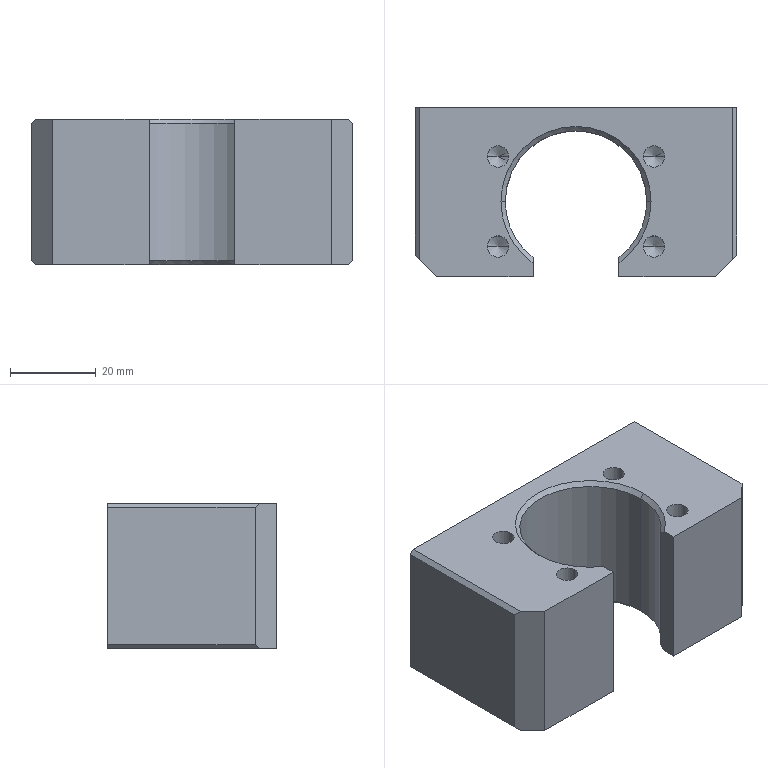Part | SolidWorks | features HoleWzd 3, Chamfer 2, ICE 2, Extrusion 1 | 1 solid | 56 faces | box 75 x 39.5 x 34 mm | volume 65045 mm3 | cone 22 | cylinder 19 | plane 15 | commonest cylinder face diameters 5 x8 6.8 x8 33 x3
STEP:
#1=CARTESIAN_POINT('',(-20.687,8.25,19.));
#2=VERTEX_POINT('',#1);
#3=CARTESIAN_POINT('',(-15.687,8.25,19.));
#4=VERTEX_POINT('',#3);
#5=CARTESIAN_POINT('',(-18.187,8.25,19.));
#6=DIRECTION('',(0.,0.,1.));
#7=DIRECTION('',(1.,0.,0.));
#8=AXIS2_PLACEMENT_3D('',#5,#6,#7);
#9=CIRCLE('',#8,2.5);
#10=EDGE_CURVE('',#2,#4,#9,.T.);
#11=ORIENTED_EDGE('',*,*,#10,.F.);
#12=CARTESIAN_POINT('',(-20.687,8.25,34.));
#13=VERTEX_POINT('',#12);
#14=CARTESIAN_POINT('',(-20.687,8.25,34.));
#15=DIRECTION('',(0.,0.,1.));
#16=VECTOR('',#15,1000.);
#17=LINE('',#14,#16);
#18=EDGE_CURVE('',#2,#13,#17,.T.);
#19=ORIENTED_EDGE('',*,*,#18,.T.);
#20=CARTESIAN_POINT('',(-15.687,8.25,34.));
#21=VERTEX_POINT('',#20);
#22=CARTESIAN_POINT('',(-18.187,8.25,34.));
#23=DIRECTION('',(0.,0.,1.));
#24=DIRECTION('',(1.,0.,0.));
#25=AXIS2_PLACEMENT_3D('',#22,#23,#24);
#26=CIRCLE('',#25,2.5);
#27=EDGE_CURVE('',#13,#21,#26,.T.);
#28=ORIENTED_EDGE('',*,*,#27,.T.);
#29=CARTESIAN_POINT('',(-15.687,8.25,34.));
#30=DIRECTION('',(0.,0.,1.));
#31=VECTOR('',#30,1000.);
#32=LINE('',#29,#31);
#33=EDGE_CURVE('',#4,#21,#32,.T.);
#34=ORIENTED_EDGE('',*,*,#33,.F.);
#35=EDGE_LOOP('',(#11,#19,#28,#34));
#36=FACE_OUTER_BOUND('',#35,.T.);
#37=CARTESIAN_POINT('',(-18.187,8.25,34.));
#38=DIRECTION('',(0.,0.,1.));
#39=DIRECTION('',(1.,0.,0.));
#40=AXIS2_PLACEMENT_3D('',#37,#38,#39);
#41=CYLINDRICAL_SURFACE('',#40,2.5);
#42=ADVANCED_FACE('',(#36),#41,.F.);
#43=CARTESIAN_POINT('',(-18.187,8.25,17.498));
#44=VERTEX_POINT('',#43);
#45=CARTESIAN_POINT('',(-15.687,8.25,19.));
#46=DIRECTION('',(0.8572,0.,0.515));
#47=VECTOR('',#46,1000.);
#48=LINE('',#45,#47);
#49=EDGE_CURVE('',#44,#4,#48,.T.);
#50=ORIENTED_EDGE('',*,*,#49,.F.);
#51=CARTESIAN_POINT('',(-20.687,8.25,19.));
#52=DIRECTION('',(-0.8572,0.,0.515));
#53=VECTOR('',#52,1000.);
#54=LINE('',#51,#53);
#55=EDGE_CURVE('',#44,#2,#54,.T.);
#56=ORIENTED_EDGE('',*,*,#55,.T.);
#57=ORIENTED_EDGE('',*,*,#10,.T.);
#58=EDGE_LOOP('',(#50,#56,#57));
#59=FACE_OUTER_BOUND('',#58,.T.);
#60=CARTESIAN_POINT('',(-18.187,8.25,19.));
#61=DIRECTION('',(0.,0.,1.));
#62=DIRECTION('',(1.,0.,0.));
#63=AXIS2_PLACEMENT_3D('',#60,#61,#62);
#64=CONICAL_SURFACE('',#63,2.5,1.03);
#65=ADVANCED_FACE('',(#59),#64,.F.);
#66=CARTESIAN_POINT('',(-20.687,-12.75,19.));
#67=VERTEX_POINT('',#66);
#68=CARTESIAN_POINT('',(-15.687,-12.75,19.));
#69=VERTEX_POINT('',#68);
#70=CARTESIAN_POINT('',(-18.187,-12.75,19.));
#71=DIRECTION('',(0.,0.,1.));
#72=DIRECTION('',(1.,0.,0.));
#73=AXIS2_PLACEMENT_3D('',#70,#71,#72);
#74=CIRCLE('',#73,2.5);
#75=EDGE_CURVE('',#67,#69,#74,.T.);
#76=ORIENTED_EDGE('',*,*,#75,.F.);
#77=CARTESIAN_POINT('',(-20.687,-12.75,34.));
#78=VERTEX_POINT('',#77);
#79=CARTESIAN_POINT('',(-20.687,-12.75,34.));
#80=DIRECTION('',(0.,0.,1.));
#81=VECTOR('',#80,1000.);
#82=LINE('',#79,#81);
#83=EDGE_CURVE('',#67,#78,#82,.T.);
#84=ORIENTED_EDGE('',*,*,#83,.T.);
#85=CARTESIAN_POINT('',(-15.687,-12.75,34.));
#86=VERTEX_POINT('',#85);
#87=CARTESIAN_POINT('',(-18.187,-12.75,34.));
#88=DIRECTION('',(0.,0.,1.));
#89=DIRECTION('',(1.,0.,0.));
#90=AXIS2_PLACEMENT_3D('',#87,#88,#89);
#91=CIRCLE('',#90,2.5);
#92=EDGE_CURVE('',#78,#86,#91,.T.);
#93=ORIENTED_EDGE('',*,*,#92,.T.);
#94=CARTESIAN_POINT('',(-15.687,-12.75,34.));
#95=DIRECTION('',(0.,0.,1.));
#96=VECTOR('',#95,1000.);
#97=LINE('',#94,#96);
#98=EDGE_CURVE('',#69,#86,#97,.T.);
#99=ORIENTED_EDGE('',*,*,#98,.F.);
#100=EDGE_LOOP('',(#76,#84,#93,#99));
#101=FACE_OUTER_BOUND('',#100,.T.);
#102=CARTESIAN_POINT('',(-18.187,-12.75,34.));
#103=DIRECTION('',(0.,0.,1.));
#104=DIRECTION('',(1.,0.,0.));
#105=AXIS2_PLACEMENT_3D('',#102,#103,#104);
#106=CYLINDRICAL_SURFACE('',#105,2.5);
#107=ADVANCED_FACE('',(#101),#106,.F.);
#108=CARTESIAN_POINT('',(-18.187,-12.75,17.498));
#109=VERTEX_POINT('',#108);
#110=CARTESIAN_POINT('',(-15.687,-12.75,19.));
#111=DIRECTION('',(0.8572,0.,0.515));
#112=VECTOR('',#111,1000.);
#113=LINE('',#110,#112);
#114=EDGE_CURVE('',#109,#69,#113,.T.);
#115=ORIENTED_EDGE('',*,*,#114,.F.);
#116=CARTESIAN_POINT('',(-20.687,-12.75,19.));
#117=DIRECTION('',(-0.8572,0.,0.515));
#118=VECTOR('',#117,1000.);
#119=LINE('',#116,#118);
#120=EDGE_CURVE('',#109,#67,#119,.T.);
#121=ORIENTED_EDGE('',*,*,#120,.T.);
#122=ORIENTED_EDGE('',*,*,#75,.T.);
#123=EDGE_LOOP('',(#115,#121,#122));
#124=FACE_OUTER_BOUND('',#123,.T.);
#125=CARTESIAN_POINT('',(-18.187,-12.75,19.));
#126=DIRECTION('',(0.,0.,1.));
#127=DIRECTION('',(1.,0.,0.));
#128=AXIS2_PLACEMENT_3D('',#125,#126,#127);
#129=CONICAL_SURFACE('',#128,2.5,1.03);
#130=ADVANCED_FACE('',(#124),#129,.F.);
#131=CARTESIAN_POINT('',(15.687,8.25,19.));
#132=VERTEX_POINT('',#131);
#133=CARTESIAN_POINT('',(20.687,8.25,19.));
#134=VERTEX_POINT('',#133);
#135=CARTESIAN_POINT('',(18.187,8.25,19.));
#136=DIRECTION('',(0.,0.,1.));
#137=DIRECTION('',(1.,0.,0.));
#138=AXIS2_PLACEMENT_3D('',#135,#136,#137);
#139=CIRCLE('',#138,2.5);
#140=EDGE_CURVE('',#132,#134,#139,.T.);
#141=ORIENTED_EDGE('',*,*,#140,.F.);
#142=CARTESIAN_POINT('',(15.687,8.25,34.));
#143=VERTEX_POINT('',#142);
#144=CARTESIAN_POINT('',(15.687,8.25,34.));
#145=DIRECTION('',(0.,0.,1.));
#146=VECTOR('',#145,1000.);
#147=LINE('',#144,#146);
#148=EDGE_CURVE('',#132,#143,#147,.T.);
#149=ORIENTED_EDGE('',*,*,#148,.T.);
#150=CARTESIAN_POINT('',(20.687,8.25,34.));
#151=VERTEX_POINT('',#150);
#152=CARTESIAN_POINT('',(18.187,8.25,34.));
#153=DIRECTION('',(0.,0.,1.));
#154=DIRECTION('',(1.,0.,0.));
#155=AXIS2_PLACEMENT_3D('',#152,#153,#154);
#156=CIRCLE('',#155,2.5);
#157=EDGE_CURVE('',#143,#151,#156,.T.);
#158=ORIENTED_EDGE('',*,*,#157,.T.);
#159=CARTESIAN_POINT('',(20.687,8.25,34.));
#160=DIRECTION('',(0.,0.,1.));
#161=VECTOR('',#160,1000.);
#162=LINE('',#159,#161);
#163=EDGE_CURVE('',#134,#151,#162,.T.);
#164=ORIENTED_EDGE('',*,*,#163,.F.);
#165=EDGE_LOOP('',(#141,#149,#158,#164));
#166=FACE_OUTER_BOUND('',#165,.T.);
#167=CARTESIAN_POINT('',(18.187,8.25,34.));
#168=DIRECTION('',(0.,0.,1.));
#169=DIRECTION('',(1.,0.,0.));
#170=AXIS2_PLACEMENT_3D('',#167,#168,#169);
#171=CYLINDRICAL_SURFACE('',#170,2.5);
#172=ADVANCED_FACE('',(#166),#171,.F.);
#173=CARTESIAN_POINT('',(18.187,8.25,17.498));
#174=VERTEX_POINT('',#173);
#175=CARTESIAN_POINT('',(20.687,8.25,19.));
#176=DIRECTION('',(0.8572,0.,0.515));
#177=VECTOR('',#176,1000.);
#178=LINE('',#175,#177);
#179=EDGE_CURVE('',#174,#134,#178,.T.);
#180=ORIENTED_EDGE('',*,*,#179,.F.);
#181=CARTESIAN_POINT('',(15.687,8.25,19.));
#182=DIRECTION('',(-0.8572,0.,0.515));
#183=VECTOR('',#182,1000.);
#184=LINE('',#181,#183);
#185=EDGE_CURVE('',#174,#132,#184,.T.);
#186=ORIENTED_EDGE('',*,*,#185,.T.);
#187=ORIENTED_EDGE('',*,*,#140,.T.);
#188=EDGE_LOOP('',(#180,#186,#187));
#189=FACE_OUTER_BOUND('',#188,.T.);
#190=CARTESIAN_POINT('',(18.187,8.25,19.));
#191=DIRECTION('',(0.,0.,1.));
#192=DIRECTION('',(1.,0.,0.));
#193=AXIS2_PLACEMENT_3D('',#190,#191,#192);
#194=CONICAL_SURFACE('',#193,2.5,1.03);
#195=ADVANCED_FACE('',(#189),#194,.F.);
#196=CARTESIAN_POINT('',(15.687,-12.75,19.));
#197=VERTEX_POINT('',#196);
#198=CARTESIAN_POINT('',(20.687,-12.75,19.));
#199=VERTEX_POINT('',#198);
#200=CARTESIAN_POINT('',(18.187,-12.75,19.));
#201=DIRECTION('',(0.,0.,1.));
#202=DIRECTION('',(1.,0.,0.));
#203=AXIS2_PLACEMENT_3D('',#200,#201,#202);
#204=CIRCLE('',#203,2.5);
#205=EDGE_CURVE('',#197,#199,#204,.T.);
#206=ORIENTED_EDGE('',*,*,#205,.F.);
#207=CARTESIAN_POINT('',(15.687,-12.75,34.));
#208=VERTEX_POINT('',#207);
#209=CARTESIAN_POINT('',(15.687,-12.75,34.));
#210=DIRECTION('',(0.,0.,1.));
#211=VECTOR('',#210,1000.);
#212=LINE('',#209,#211);
#213=EDGE_CURVE('',#197,#208,#212,.T.);
#214=ORIENTED_EDGE('',*,*,#213,.T.);
#215=CARTESIAN_POINT('',(20.687,-12.75,34.));
#216=VERTEX_POINT('',#215);
#217=CARTESIAN_POINT('',(18.187,-12.75,34.));
#218=DIRECTION('',(0.,0.,1.));
#219=DIRECTION('',(1.,0.,0.));
#220=AXIS2_PLACEMENT_3D('',#217,#218,#219);
#221=CIRCLE('',#220,2.5);
#222=EDGE_CURVE('',#208,#216,#221,.T.);
#223=ORIENTED_EDGE('',*,*,#222,.T.);
#224=CARTESIAN_POINT('',(20.687,-12.75,34.));
#225=DIRECTION('',(0.,0.,1.));
#226=VECTOR('',#225,1000.);
#227=LINE('',#224,#226);
#228=EDGE_CURVE('',#199,#216,#227,.T.);
#229=ORIENTED_EDGE('',*,*,#228,.F.);
#230=EDGE_LOOP('',(#206,#214,#223,#229));
#231=FACE_OUTER_BOUND('',#230,.T.);
#232=CARTESIAN_POINT('',(18.187,-12.75,34.));
#233=DIRECTION('',(0.,0.,1.));
#234=DIRECTION('',(1.,0.,0.));
#235=AXIS2_PLACEMENT_3D('',#232,#233,#234);
#236=CYLINDRICAL_SURFACE('',#235,2.5);
#237=ADVANCED_FACE('',(#231),#236,.F.);
#238=CARTESIAN_POINT('',(18.187,-12.75,17.498));
#239=VERTEX_POINT('',#238);
#240=CARTESIAN_POINT('',(20.687,-12.75,19.));
#241=DIRECTION('',(0.8572,0.,0.515));
#242=VECTOR('',#241,1000.);
#243=LINE('',#240,#242);
#244=EDGE_CURVE('',#239,#199,#243,.T.);
#245=ORIENTED_EDGE('',*,*,#244,.F.);
#246=CARTESIAN_POINT('',(15.687,-12.75,19.));
#247=DIRECTION('',(-0.8572,0.,0.515));
#248=VECTOR('',#247,1000.);
#249=LINE('',#246,#248);
#250=EDGE_CURVE('',#239,#197,#249,.T.);
#251=ORIENTED_EDGE('',*,*,#250,.T.);
#252=ORIENTED_EDGE('',*,*,#205,.T.);
#253=EDGE_LOOP('',(#245,#251,#252));
#254=FACE_OUTER_BOUND('',#253,.T.);
#255=CARTESIAN_POINT('',(18.187,-12.75,19.));
#256=DIRECTION('',(0.,0.,1.));
#257=DIRECTION('',(1.,0.,0.));
#258=AXIS2_PLACEMENT_3D('',#255,#256,#257);
#259=CONICAL_SURFACE('',#258,2.5,1.03);
#260=ADVANCED_FACE('',(#254),#259,.F.);
#261=CARTESIAN_POINT('',(-16.5,-2.25,33.));
#262=VERTEX_POINT('',#261);
#263=CARTESIAN_POINT('',(-10.,-15.374,33.));
#264=VERTEX_POINT('',#263);
#265=CARTESIAN_POINT('',(0.,-2.25,33.));
#266=DIRECTION('',(0.,0.,1.));
#267=DIRECTION('',(-1.,0.,0.));
#268=AXIS2_PLACEMENT_3D('',#265,#266,#267);
#269=CIRCLE('',#268,16.5);
#270=EDGE_CURVE('',#262,#264,#269,.T.);
#271=ORIENTED_EDGE('',*,*,#270,.F.);
#272=CARTESIAN_POINT('',(-17.5,-2.25,34.));
#273=VERTEX_POINT('',#272);
#274=CARTESIAN_POINT('',(-16.5,-2.25,33.));
#275=DIRECTION('',(-0.7071,0.,0.7071));
#276=VECTOR('',#275,1000.);
#277=LINE('',#274,#276);
#278=EDGE_CURVE('',#262,#273,#277,.T.);
#279=ORIENTED_EDGE('',*,*,#278,.T.);
#280=CARTESIAN_POINT('',(-10.,-16.611,34.));
#281=VERTEX_POINT('',#280);
#282=CARTESIAN_POINT('',(0.,-2.25,34.));
#283=DIRECTION('',(0.,0.,-1.));
#284=DIRECTION('',(-1.,0.,0.));
#285=AXIS2_PLACEMENT_3D('',#282,#283,#284);
#286=CIRCLE('',#285,17.5);
#287=EDGE_CURVE('',#281,#273,#286,.T.);
#288=ORIENTED_EDGE('',*,*,#287,.F.);
#289=CARTESIAN_POINT('',(-10.,-15.374,33.));
#290=CARTESIAN_POINT('',(-10.,-15.789,33.33));
#291=CARTESIAN_POINT('',(-10.,-16.202,33.664));
#292=CARTESIAN_POINT('',(-10.,-16.611,34.));
#293=B_SPLINE_CURVE_WITH_KNOTS('',3,(#289,#290,#291,#292),.UNSPECIFIED.,.F.,.F.,(4,4),(0.,0.001591),.UNSPECIFIED.);
#294=EDGE_CURVE('',#264,#281,#293,.T.);
#295=ORIENTED_EDGE('',*,*,#294,.F.);
#296=EDGE_LOOP('',(#271,#279,#288,#295));
#297=FACE_OUTER_BOUND('',#296,.T.);
#298=CARTESIAN_POINT('',(0.,-2.25,33.));
#299=DIRECTION('',(0.,0.,1.));
#300=DIRECTION('',(1.,0.,0.));
#301=AXIS2_PLACEMENT_3D('',#298,#299,#300);
#302=CONICAL_SURFACE('',#301,16.5,0.7854);
#303=ADVANCED_FACE('',(#297),#302,.F.);
#304=ORIENTED_EDGE('',*,*,#278,.F.);
#305=CARTESIAN_POINT('',(16.5,-2.25,33.));
#306=VERTEX_POINT('',#305);
#307=CARTESIAN_POINT('',(0.,-2.25,33.));
#308=DIRECTION('',(0.,0.,1.));
#309=DIRECTION('',(-1.,0.,0.));
#310=AXIS2_PLACEMENT_3D('',#307,#308,#309);
#311=CIRCLE('',#310,16.5);
#312=EDGE_CURVE('',#306,#262,#311,.T.);
#313=ORIENTED_EDGE('',*,*,#312,.F.);
#314=CARTESIAN_POINT('',(17.5,-2.25,34.));
#315=VERTEX_POINT('',#314);
#316=CARTESIAN_POINT('',(16.5,-2.25,33.));
#317=DIRECTION('',(0.7071,0.,0.7071));
#318=VECTOR('',#317,1000.);
#319=LINE('',#316,#318);
#320=EDGE_CURVE('',#306,#315,#319,.T.);
#321=ORIENTED_EDGE('',*,*,#320,.T.);
#322=CARTESIAN_POINT('',(0.,-2.25,34.));
#323=DIRECTION('',(0.,0.,-1.));
#324=DIRECTION('',(-1.,0.,0.));
#325=AXIS2_PLACEMENT_3D('',#322,#323,#324);
#326=CIRCLE('',#325,17.5);
#327=EDGE_CURVE('',#273,#315,#326,.T.);
#328=ORIENTED_EDGE('',*,*,#327,.F.);
#329=EDGE_LOOP('',(#304,#313,#321,#328));
#330=FACE_OUTER_BOUND('',#329,.T.);
#331=CARTESIAN_POINT('',(0.,-2.25,33.));
#332=DIRECTION('',(0.,0.,1.));
#333=DIRECTION('',(1.,0.,0.));
#334=AXIS2_PLACEMENT_3D('',#331,#332,#333);
#335=CONICAL_SURFACE('',#334,16.5,0.7854);
#336=ADVANCED_FACE('',(#330),#335,.F.);
#337=CARTESIAN_POINT('',(16.5,-2.25,1.));
#338=VERTEX_POINT('',#337);
#339=CARTESIAN_POINT('',(10.,-15.374,1.));
#340=VERTEX_POINT('',#339);
#341=CARTESIAN_POINT('',(0.,-2.25,1.));
#342=DIRECTION('',(0.,0.,-1.));
#343=DIRECTION('',(-1.,0.,0.));
#344=AXIS2_PLACEMENT_3D('',#341,#342,#343);
#345=CIRCLE('',#344,16.5);
#346=EDGE_CURVE('',#338,#340,#345,.T.);
#347=ORIENTED_EDGE('',*,*,#346,.F.);
#348=CARTESIAN_POINT('',(17.5,-2.25,0.));
#349=VERTEX_POINT('',#348);
#350=CARTESIAN_POINT('',(17.5,-2.25,0.));
#351=DIRECTION('',(0.7071,0.,-0.7071));
#352=VECTOR('',#351,1000.);
#353=LINE('',#350,#352);
#354=EDGE_CURVE('',#338,#349,#353,.T.);
#355=ORIENTED_EDGE('',*,*,#354,.T.);
#356=CARTESIAN_POINT('',(10.,-16.611,0.));
#357=VERTEX_POINT('',#356);
#358=CARTESIAN_POINT('',(0.,-2.25,0.));
#359=DIRECTION('',(0.,0.,1.));
#360=DIRECTION('',(-1.,0.,0.));
#361=AXIS2_PLACEMENT_3D('',#358,#359,#360);
#362=CIRCLE('',#361,17.5);
#363=EDGE_CURVE('',#357,#349,#362,.T.);
#364=ORIENTED_EDGE('',*,*,#363,.F.);
#365=CARTESIAN_POINT('',(10.,-15.374,1.));
#366=CARTESIAN_POINT('',(10.,-15.789,0.6699));
#367=CARTESIAN_POINT('',(10.,-16.202,0.3364));
#368=CARTESIAN_POINT('',(10.,-16.611,0.));
#369=B_SPLINE_CURVE_WITH_KNOTS('',3,(#365,#366,#367,#368),.UNSPECIFIED.,.F.,.F.,(4,4),(0.,0.001591),.UNSPECIFIED.);
#370=EDGE_CURVE('',#340,#357,#369,.T.);
#371=ORIENTED_EDGE('',*,*,#370,.F.);
#372=EDGE_LOOP('',(#347,#355,#364,#371));
#373=FACE_OUTER_BOUND('',#372,.T.);
#374=CARTESIAN_POINT('',(0.,-2.25,0.));
#375=DIRECTION('',(0.,0.,-1.));
#376=DIRECTION('',(-1.,0.,0.));
#377=AXIS2_PLACEMENT_3D('',#374,#375,#376);
#378=CONICAL_SURFACE('',#377,17.5,0.7854);
#379=ADVANCED_FACE('',(#373),#378,.F.);
#380=ORIENTED_EDGE('',*,*,#354,.F.);
#381=CARTESIAN_POINT('',(-16.5,-2.25,1.));
#382=VERTEX_POINT('',#381);
#383=CARTESIAN_POINT('',(0.,-2.25,1.));
#384=DIRECTION('',(0.,0.,-1.));
#385=DIRECTION('',(-1.,0.,0.));
#386=AXIS2_PLACEMENT_3D('',#383,#384,#385);
#387=CIRCLE('',#386,16.5);
#388=EDGE_CURVE('',#382,#338,#387,.T.);
#389=ORIENTED_EDGE('',*,*,#388,.F.);
#390=CARTESIAN_POINT('',(-17.5,-2.25,0.));
#391=VERTEX_POINT('',#390);
#392=CARTESIAN_POINT('',(-17.5,-2.25,0.));
#393=DIRECTION('',(-0.7071,0.,-0.7071));
#394=VECTOR('',#393,1000.);
#395=LINE('',#392,#394);
#396=EDGE_CURVE('',#382,#391,#395,.T.);
#397=ORIENTED_EDGE('',*,*,#396,.T.);
#398=CARTESIAN_POINT('',(0.,-2.25,0.));
#399=DIRECTION('',(0.,0.,1.));
#400=DIRECTION('',(-1.,0.,0.));
#401=AXIS2_PLACEMENT_3D('',#398,#399,#400);
#402=CIRCLE('',#401,17.5);
#403=EDGE_CURVE('',#349,#391,#402,.T.);
#404=ORIENTED_EDGE('',*,*,#403,.F.);
#405=EDGE_LOOP('',(#380,#389,#397,#404));
#406=FACE_OUTER_BOUND('',#405,.T.);
#407=CARTESIAN_POINT('',(0.,-2.25,0.));
#408=DIRECTION('',(0.,0.,-1.));
#409=DIRECTION('',(-1.,0.,0.));
#410=AXIS2_PLACEMENT_3D('',#407,#408,#409);
#411=CONICAL_SURFACE('',#410,17.5,0.7854);
#412=ADVANCED_FACE('',(#406),#411,.F.);
#413=CARTESIAN_POINT('',(-27.5,0.,3.6));
#414=VERTEX_POINT('',#413);
#415=CARTESIAN_POINT('',(-27.5,0.,10.4));
#416=VERTEX_POINT('',#415);
#417=CARTESIAN_POINT('',(-27.5,0.,7.));
#418=DIRECTION('',(0.,1.,0.));
#419=DIRECTION('',(0.,0.,1.));
#420=AXIS2_PLACEMENT_3D('',#417,#418,#419);
#421=CIRCLE('',#420,3.4);
#422=EDGE_CURVE('',#414,#416,#421,.T.);
#423=ORIENTED_EDGE('',*,*,#422,.F.);
#424=CARTESIAN_POINT('',(-27.5,19.75,3.6));
#425=VERTEX_POINT('',#424);
#426=CARTESIAN_POINT('',(-27.5,19.75,3.6));
#427=DIRECTION('',(0.,1.,0.));
#428=VECTOR('',#427,1000.);
#429=LINE('',#426,#428);
#430=EDGE_CURVE('',#414,#425,#429,.T.);
#431=ORIENTED_EDGE('',*,*,#430,.T.);
#432=CARTESIAN_POINT('',(-27.5,19.75,10.4));
#433=VERTEX_POINT('',#432);
#434=CARTESIAN_POINT('',(-27.5,19.75,7.));
#435=DIRECTION('',(0.,1.,0.));
#436=DIRECTION('',(0.,0.,1.));
#437=AXIS2_PLACEMENT_3D('',#434,#435,#436);
#438=CIRCLE('',#437,3.4);
#439=EDGE_CURVE('',#425,#433,#438,.T.);
#440=ORIENTED_EDGE('',*,*,#439,.T.);
#441=CARTESIAN_POINT('',(-27.5,19.75,10.4));
#442=DIRECTION('',(0.,1.,0.));
#443=VECTOR('',#442,1000.);
#444=LINE('',#441,#443);
#445=EDGE_CURVE('',#416,#433,#444,.T.);
#446=ORIENTED_EDGE('',*,*,#445,.F.);
#447=EDGE_LOOP('',(#423,#431,#440,#446));
#448=FACE_OUTER_BOUND('',#447,.T.);
#449=CARTESIAN_POINT('',(-27.5,19.75,7.));
#450=DIRECTION('',(0.,1.,0.));
#451=DIRECTION('',(0.,0.,1.));
#452=AXIS2_PLACEMENT_3D('',#449,#450,#451);
#453=CYLINDRICAL_SURFACE('',#452,3.4);
#454=ADVANCED_FACE('',(#448),#453,.F.);
#455=CARTESIAN_POINT('',(-27.5,-2.043,7.));
#456=VERTEX_POINT('',#455);
#457=CARTESIAN_POINT('',(-27.5,0.,10.4));
#458=DIRECTION('',(0.,0.515,0.8572));
#459=VECTOR('',#458,1000.);
#460=LINE('',#457,#459);
#461=EDGE_CURVE('',#456,#416,#460,.T.);
#462=ORIENTED_EDGE('',*,*,#461,.F.);
#463=CARTESIAN_POINT('',(-27.5,0.,3.6));
#464=DIRECTION('',(0.,0.515,-0.8572));
#465=VECTOR('',#464,1000.);
#466=LINE('',#463,#465);
#467=EDGE_CURVE('',#456,#414,#466,.T.);
#468=ORIENTED_EDGE('',*,*,#467,.T.);
#469=ORIENTED_EDGE('',*,*,#422,.T.);
#470=EDGE_LOOP('',(#462,#468,#469));
#471=FACE_OUTER_BOUND('',#470,.T.);
#472=CARTESIAN_POINT('',(-27.5,0.,7.));
#473=DIRECTION('',(0.,1.,0.));
#474=DIRECTION('',(0.,0.,1.));
#475=AXIS2_PLACEMENT_3D('',#472,#473,#474);
#476=CONICAL_SURFACE('',#475,3.4,1.03);
#477=ADVANCED_FACE('',(#471),#476,.F.);
#478=CARTESIAN_POINT('',(-27.5,0.,23.6));
#479=VERTEX_POINT('',#478);
#480=CARTESIAN_POINT('',(-27.5,0.,30.4));
#481=VERTEX_POINT('',#480);
#482=CARTESIAN_POINT('',(-27.5,0.,27.));
#483=DIRECTION('',(0.,1.,0.));
#484=DIRECTION('',(0.,0.,1.));
#485=AXIS2_PLACEMENT_3D('',#482,#483,#484);
#486=CIRCLE('',#485,3.4);
#487=EDGE_CURVE('',#479,#481,#486,.T.);
#488=ORIENTED_EDGE('',*,*,#487,.F.);
#489=CARTESIAN_POINT('',(-27.5,19.75,23.6));
#490=VERTEX_POINT('',#489);
#491=CARTESIAN_POINT('',(-27.5,19.75,23.6));
#492=DIRECTION('',(0.,1.,0.));
#493=VECTOR('',#492,1000.);
#494=LINE('',#491,#493);
#495=EDGE_CURVE('',#479,#490,#494,.T.);
#496=ORIENTED_EDGE('',*,*,#495,.T.);
#497=CARTESIAN_POINT('',(-27.5,19.75,30.4));
#498=VERTEX_POINT('',#497);
#499=CARTESIAN_POINT('',(-27.5,19.75,27.));
#500=DIRECTION('',(0.,1.,0.));
#501=DIRECTION('',(0.,0.,1.));
#502=AXIS2_PLACEMENT_3D('',#499,#500,#501);
#503=CIRCLE('',#502,3.4);
#504=EDGE_CURVE('',#490,#498,#503,.T.);
#505=ORIENTED_EDGE('',*,*,#504,.T.);
#506=CARTESIAN_POINT('',(-27.5,19.75,30.4));
#507=DIRECTION('',(0.,1.,0.));
#508=VECTOR('',#507,1000.);
#509=LINE('',#506,#508);
#510=EDGE_CURVE('',#481,#498,#509,.T.);
#511=ORIENTED_EDGE('',*,*,#510,.F.);
#512=EDGE_LOOP('',(#488,#496,#505,#511));
#513=FACE_OUTER_BOUND('',#512,.T.);
#514=CARTESIAN_POINT('',(-27.5,19.75,27.));
#515=DIRECTION('',(0.,1.,0.));
#516=DIRECTION('',(0.,0.,1.));
#517=AXIS2_PLACEMENT_3D('',#514,#515,#516);
#518=CYLINDRICAL_SURFACE('',#517,3.4);
#519=ADVANCED_FACE('',(#513),#518,.F.);
#520=CARTESIAN_POINT('',(-27.5,-2.043,27.));
#521=VERTEX_POINT('',#520);
#522=CARTESIAN_POINT('',(-27.5,0.,30.4));
#523=DIRECTION('',(0.,0.515,0.8572));
#524=VECTOR('',#523,1000.);
#525=LINE('',#522,#524);
#526=EDGE_CURVE('',#521,#481,#525,.T.);
#527=ORIENTED_EDGE('',*,*,#526,.F.);
#528=CARTESIAN_POINT('',(-27.5,0.,23.6));
#529=DIRECTION('',(0.,0.515,-0.8572));
#530=VECTOR('',#529,1000.);
#531=LINE('',#528,#530);
#532=EDGE_CURVE('',#521,#479,#531,.T.);
#533=ORIENTED_EDGE('',*,*,#532,.T.);
#534=ORIENTED_EDGE('',*,*,#487,.T.);
#535=EDGE_LOOP('',(#527,#533,#534));
#536=FACE_OUTER_BOUND('',#535,.T.);
#537=CARTESIAN_POINT('',(-27.5,0.,27.));
#538=DIRECTION('',(0.,1.,0.));
#539=DIRECTION('',(0.,0.,1.));
#540=AXIS2_PLACEMENT_3D('',#537,#538,#539);
#541=CONICAL_SURFACE('',#540,3.4,1.03);
#542=ADVANCED_FACE('',(#536),#541,.F.);
#543=CARTESIAN_POINT('',(27.5,0.,23.6));
#544=VERTEX_POINT('',#543);
#545=CARTESIAN_POINT('',(27.5,0.,30.4));
#546=VERTEX_POINT('',#545);
#547=CARTESIAN_POINT('',(27.5,0.,27.));
#548=DIRECTION('',(0.,1.,0.));
#549=DIRECTION('',(0.,0.,1.));
#550=AXIS2_PLACEMENT_3D('',#547,#548,#549);
#551=CIRCLE('',#550,3.4);
#552=EDGE_CURVE('',#544,#546,#551,.T.);
#553=ORIENTED_EDGE('',*,*,#552,.F.);
#554=CARTESIAN_POINT('',(27.5,19.75,23.6));
#555=VERTEX_POINT('',#554);
#556=CARTESIAN_POINT('',(27.5,19.75,23.6));
#557=DIRECTION('',(0.,1.,0.));
#558=VECTOR('',#557,1000.);
#559=LINE('',#556,#558);
#560=EDGE_CURVE('',#544,#555,#559,.T.);
#561=ORIENTED_EDGE('',*,*,#560,.T.);
#562=CARTESIAN_POINT('',(27.5,19.75,30.4));
#563=VERTEX_POINT('',#562);
#564=CARTESIAN_POINT('',(27.5,19.75,27.));
#565=DIRECTION('',(0.,1.,0.));
#566=DIRECTION('',(0.,0.,1.));
#567=AXIS2_PLACEMENT_3D('',#564,#565,#566);
#568=CIRCLE('',#567,3.4);
#569=EDGE_CURVE('',#555,#563,#568,.T.);
#570=ORIENTED_EDGE('',*,*,#569,.T.);
#571=CARTESIAN_POINT('',(27.5,19.75,30.4));
#572=DIRECTION('',(0.,1.,0.));
#573=VECTOR('',#572,1000.);
#574=LINE('',#571,#573);
#575=EDGE_CURVE('',#546,#563,#574,.T.);
#576=ORIENTED_EDGE('',*,*,#575,.F.);
#577=EDGE_LOOP('',(#553,#561,#570,#576));
#578=FACE_OUTER_BOUND('',#577,.T.);
#579=CARTESIAN_POINT('',(27.5,19.75,27.));
#580=DIRECTION('',(0.,1.,0.));
#581=DIRECTION('',(0.,0.,1.));
#582=AXIS2_PLACEMENT_3D('',#579,#580,#581);
#583=CYLINDRICAL_SURFACE('',#582,3.4);
#584=ADVANCED_FACE('',(#578),#583,.F.);
#585=CARTESIAN_POINT('',(27.5,-2.043,27.));
#586=VERTEX_POINT('',#585);
#587=CARTESIAN_POINT('',(27.5,0.,30.4));
#588=DIRECTION('',(0.,0.515,0.8572));
#589=VECTOR('',#588,1000.);
#590=LINE('',#587,#589);
#591=EDGE_CURVE('',#586,#546,#590,.T.);
#592=ORIENTED_EDGE('',*,*,#591,.F.);
#593=CARTESIAN_POINT('',(27.5,0.,23.6));
#594=DIRECTION('',(0.,0.515,-0.8572));
#595=VECTOR('',#594,1000.);
#596=LINE('',#593,#595);
#597=EDGE_CURVE('',#586,#544,#596,.T.);
#598=ORIENTED_EDGE('',*,*,#597,.T.);
#599=ORIENTED_EDGE('',*,*,#552,.T.);
#600=EDGE_LOOP('',(#592,#598,#599));
#601=FACE_OUTER_BOUND('',#600,.T.);
#602=CARTESIAN_POINT('',(27.5,0.,27.));
#603=DIRECTION('',(0.,1.,0.));
#604=DIRECTION('',(0.,0.,1.));
#605=AXIS2_PLACEMENT_3D('',#602,#603,#604);
#606=CONICAL_SURFACE('',#605,3.4,1.03);
#607=ADVANCED_FACE('',(#601),#606,.F.);
#608=CARTESIAN_POINT('',(27.5,0.,3.6));
#609=VERTEX_POINT('',#608);
#610=CARTESIAN_POINT('',(27.5,0.,10.4));
#611=VERTEX_POINT('',#610);
#612=CARTESIAN_POINT('',(27.5,0.,7.));
#613=DIRECTION('',(0.,1.,0.));
#614=DIRECTION('',(0.,0.,1.));
#615=AXIS2_PLACEMENT_3D('',#612,#613,#614);
#616=CIRCLE('',#615,3.4);
#617=EDGE_CURVE('',#609,#611,#616,.T.);
#618=ORIENTED_EDGE('',*,*,#617,.F.);
#619=CARTESIAN_POINT('',(27.5,19.75,3.6));
#620=VERTEX_POINT('',#619);
#621=CARTESIAN_POINT('',(27.5,19.75,3.6));
#622=DIRECTION('',(0.,1.,0.));
#623=VECTOR('',#622,1000.);
#624=LINE('',#621,#623);
#625=EDGE_CURVE('',#609,#620,#624,.T.);
#626=ORIENTED_EDGE('',*,*,#625,.T.);
#627=CARTESIAN_POINT('',(27.5,19.75,10.4));
#628=VERTEX_POINT('',#627);
#629=CARTESIAN_POINT('',(27.5,19.75,7.));
#630=DIRECTION('',(0.,1.,0.));
#631=DIRECTION('',(0.,0.,1.));
#632=AXIS2_PLACEMENT_3D('',#629,#630,#631);
#633=CIRCLE('',#632,3.4);
#634=EDGE_CURVE('',#620,#628,#633,.T.);
#635=ORIENTED_EDGE('',*,*,#634,.T.);
#636=CARTESIAN_POINT('',(27.5,19.75,10.4));
#637=DIRECTION('',(0.,1.,0.));
#638=VECTOR('',#637,1000.);
#639=LINE('',#636,#638);
#640=EDGE_CURVE('',#611,#628,#639,.T.);
#641=ORIENTED_EDGE('',*,*,#640,.F.);
#642=EDGE_LOOP('',(#618,#626,#635,#641));
#643=FACE_OUTER_BOUND('',#642,.T.);
#644=CARTESIAN_POINT('',(27.5,19.75,7.));
#645=DIRECTION('',(0.,1.,0.));
#646=DIRECTION('',(0.,0.,1.));
#647=AXIS2_PLACEMENT_3D('',#644,#645,#646);
#648=CYLINDRICAL_SURFACE('',#647,3.4);
#649=ADVANCED_FACE('',(#643),#648,.F.);
#650=CARTESIAN_POINT('',(27.5,-2.043,7.));
#651=VERTEX_POINT('',#650);
#652=CARTESIAN_POINT('',(27.5,0.,10.4));
#653=DIRECTION('',(0.,0.515,0.8572));
#654=VECTOR('',#653,1000.);
#655=LINE('',#652,#654);
#656=EDGE_CURVE('',#651,#611,#655,.T.);
#657=ORIENTED_EDGE('',*,*,#656,.F.);
#658=CARTESIAN_POINT('',(27.5,0.,3.6));
#659=DIRECTION('',(0.,0.515,-0.8572));
#660=VECTOR('',#659,1000.);
#661=LINE('',#658,#660);
#662=EDGE_CURVE('',#651,#609,#661,.T.);
#663=ORIENTED_EDGE('',*,*,#662,.T.);
#664=ORIENTED_EDGE('',*,*,#617,.T.);
#665=EDGE_LOOP('',(#657,#663,#664));
#666=FACE_OUTER_BOUND('',#665,.T.);
#667=CARTESIAN_POINT('',(27.5,0.,7.));
#668=DIRECTION('',(0.,1.,0.));
#669=DIRECTION('',(0.,0.,1.));
#670=AXIS2_PLACEMENT_3D('',#667,#668,#669);
#671=CONICAL_SURFACE('',#670,3.4,1.03);
#672=ADVANCED_FACE('',(#666),#671,.F.);
#673=CARTESIAN_POINT('',(-10.,-15.374,1.));
#674=VERTEX_POINT('',#673);
#675=CARTESIAN_POINT('',(0.,-2.25,1.));
#676=DIRECTION('',(0.,0.,-1.));
#677=DIRECTION('',(-1.,0.,0.));
#678=AXIS2_PLACEMENT_3D('',#675,#676,#677);
#679=CIRCLE('',#678,16.5);
#680=EDGE_CURVE('',#674,#382,#679,.T.);
#681=ORIENTED_EDGE('',*,*,#680,.T.);
#682=CARTESIAN_POINT('',(-16.5,-2.25,0.));
#683=DIRECTION('',(0.,0.,1.));
#684=VECTOR('',#683,1000.);
#685=LINE('',#682,#684);
#686=EDGE_CURVE('',#382,#262,#685,.T.);
#687=ORIENTED_EDGE('',*,*,#686,.T.);
#688=ORIENTED_EDGE('',*,*,#270,.T.);
#689=CARTESIAN_POINT('',(-10.,-15.374,0.));
#690=DIRECTION('',(0.,0.,1.));
#691=VECTOR('',#690,1000.);
#692=LINE('',#689,#691);
#693=EDGE_CURVE('',#674,#264,#692,.T.);
#694=ORIENTED_EDGE('',*,*,#693,.F.);
#695=EDGE_LOOP('',(#681,#687,#688,#694));
#696=FACE_OUTER_BOUND('',#695,.T.);
#697=CARTESIAN_POINT('',(0.,-2.25,0.));
#698=DIRECTION('',(0.,0.,1.));
#699=DIRECTION('',(1.,0.,0.));
#700=AXIS2_PLACEMENT_3D('',#697,#698,#699);
#701=CYLINDRICAL_SURFACE('',#700,16.5);
#702=ADVANCED_FACE('',(#696),#701,.F.);
#703=ORIENTED_EDGE('',*,*,#686,.F.);
#704=ORIENTED_EDGE('',*,*,#388,.T.);
#705=CARTESIAN_POINT('',(16.5,-2.25,0.));
#706=DIRECTION('',(0.,0.,1.));
#707=VECTOR('',#706,1000.);
#708=LINE('',#705,#707);
#709=EDGE_CURVE('',#338,#306,#708,.T.);
#710=ORIENTED_EDGE('',*,*,#709,.T.);
#711=ORIENTED_EDGE('',*,*,#312,.T.);
#712=EDGE_LOOP('',(#703,#704,#710,#711));
#713=FACE_OUTER_BOUND('',#712,.T.);
#714=CARTESIAN_POINT('',(0.,-2.25,0.));
#715=DIRECTION('',(0.,0.,1.));
#716=DIRECTION('',(1.,0.,0.));
#717=AXIS2_PLACEMENT_3D('',#714,#715,#716);
#718=CYLINDRICAL_SURFACE('',#717,16.5);
#719=ADVANCED_FACE('',(#713),#718,.F.);
#720=CARTESIAN_POINT('',(-32.5,-19.75,34.));
#721=VERTEX_POINT('',#720);
#722=CARTESIAN_POINT('',(-10.,-19.75,34.));
#723=VERTEX_POINT('',#722);
#724=CARTESIAN_POINT('',(-37.5,-19.75,34.));
#725=DIRECTION('',(1.,0.,0.));
#726=VECTOR('',#725,1000.);
#727=LINE('',#724,#726);
#728=EDGE_CURVE('',#721,#723,#727,.T.);
#729=ORIENTED_EDGE('',*,*,#728,.F.);
#730=CARTESIAN_POINT('',(-32.5,-19.75,0.));
#731=VERTEX_POINT('',#730);
#732=CARTESIAN_POINT('',(-32.5,-19.75,34.));
#733=DIRECTION('',(0.,0.,-1.));
#734=VECTOR('',#733,1000.);
#735=LINE('',#732,#734);
#736=EDGE_CURVE('',#721,#731,#735,.T.);
#737=ORIENTED_EDGE('',*,*,#736,.T.);
#738=CARTESIAN_POINT('',(-10.,-19.75,0.));
#739=VERTEX_POINT('',#738);
#740=CARTESIAN_POINT('',(-37.5,-19.75,0.));
#741=DIRECTION('',(1.,0.,0.));
#742=VECTOR('',#741,1000.);
#743=LINE('',#740,#742);
#744=EDGE_CURVE('',#731,#739,#743,.T.);
#745=ORIENTED_EDGE('',*,*,#744,.T.);
#746=CARTESIAN_POINT('',(-10.,-19.75,0.));
#747=DIRECTION('',(0.,0.,1.));
#748=VECTOR('',#747,1000.);
#749=LINE('',#746,#748);
#750=EDGE_CURVE('',#739,#723,#749,.T.);
#751=ORIENTED_EDGE('',*,*,#750,.T.);
#752=EDGE_LOOP('',(#729,#737,#745,#751));
#753=FACE_OUTER_BOUND('',#752,.T.);
#754=CARTESIAN_POINT('',(-37.5,-19.75,34.));
#755=DIRECTION('',(0.,1.,0.));
#756=DIRECTION('',(0.,0.,1.));
#757=AXIS2_PLACEMENT_3D('',#754,#755,#756);
#758=PLANE('',#757);
#759=ADVANCED_FACE('',(#753),#758,.F.);
#760=CARTESIAN_POINT('',(37.5,19.75,33.));
#761=VERTEX_POINT('',#760);
#762=CARTESIAN_POINT('',(37.5,19.75,1.));
#763=VERTEX_POINT('',#762);
#764=CARTESIAN_POINT('',(37.5,19.75,34.));
#765=DIRECTION('',(0.,0.,-1.));
#766=VECTOR('',#765,1000.);
#767=LINE('',#764,#766);
#768=EDGE_CURVE('',#761,#763,#767,.T.);
#769=ORIENTED_EDGE('',*,*,#768,.F.);
#770=CARTESIAN_POINT('',(37.5,-14.75,33.));
#771=VERTEX_POINT('',#770);
#772=CARTESIAN_POINT('',(37.5,-19.75,33.));
#773=DIRECTION('',(0.,-1.,0.));
#774=VECTOR('',#773,1000.);
#775=LINE('',#772,#774);
#776=EDGE_CURVE('',#761,#771,#775,.T.);
#777=ORIENTED_EDGE('',*,*,#776,.T.);
#778=CARTESIAN_POINT('',(37.5,-14.75,1.));
#779=VERTEX_POINT('',#778);
#780=CARTESIAN_POINT('',(37.5,-14.75,34.));
#781=DIRECTION('',(0.,0.,-1.));
#782=VECTOR('',#781,1000.);
#783=LINE('',#780,#782);
#784=EDGE_CURVE('',#771,#779,#783,.T.);
#785=ORIENTED_EDGE('',*,*,#784,.T.);
#786=CARTESIAN_POINT('',(37.5,19.75,1.));
#787=DIRECTION('',(0.,1.,0.));
#788=VECTOR('',#787,1000.);
#789=LINE('',#786,#788);
#790=EDGE_CURVE('',#779,#763,#789,.T.);
#791=ORIENTED_EDGE('',*,*,#790,.T.);
#792=EDGE_LOOP('',(#769,#777,#785,#791));
#793=FACE_OUTER_BOUND('',#792,.T.);
#794=CARTESIAN_POINT('',(37.5,-19.75,34.));
#795=DIRECTION('',(-1.,0.,0.));
#796=DIRECTION('',(0.,0.,1.));
#797=AXIS2_PLACEMENT_3D('',#794,#795,#796);
#798=PLANE('',#797);
#799=ADVANCED_FACE('',(#793),#798,.F.);
#800=CARTESIAN_POINT('',(-27.5,19.75,7.));
#801=DIRECTION('',(0.,1.,0.));
#802=DIRECTION('',(0.,0.,1.));
#803=AXIS2_PLACEMENT_3D('',#800,#801,#802);
#804=CIRCLE('',#803,3.4);
#805=EDGE_CURVE('',#433,#425,#804,.T.);
#806=ORIENTED_EDGE('',*,*,#805,.F.);
#807=ORIENTED_EDGE('',*,*,#439,.F.);
#808=EDGE_LOOP('',(#806,#807));
#809=FACE_BOUND('',#808,.T.);
#810=CARTESIAN_POINT('',(-27.5,19.75,27.));
#811=DIRECTION('',(0.,1.,0.));
#812=DIRECTION('',(0.,0.,1.));
#813=AXIS2_PLACEMENT_3D('',#810,#811,#812);
#814=CIRCLE('',#813,3.4);
#815=EDGE_CURVE('',#498,#490,#814,.T.);
#816=ORIENTED_EDGE('',*,*,#815,.F.);
#817=ORIENTED_EDGE('',*,*,#504,.F.);
#818=EDGE_LOOP('',(#816,#817));
#819=FACE_BOUND('',#818,.T.);
#820=CARTESIAN_POINT('',(27.5,19.75,27.));
#821=DIRECTION('',(0.,1.,0.));
#822=DIRECTION('',(0.,0.,1.));
#823=AXIS2_PLACEMENT_3D('',#820,#821,#822);
#824=CIRCLE('',#823,3.4);
#825=EDGE_CURVE('',#563,#555,#824,.T.);
#826=ORIENTED_EDGE('',*,*,#825,.F.);
#827=ORIENTED_EDGE('',*,*,#569,.F.);
#828=EDGE_LOOP('',(#826,#827));
#829=FACE_BOUND('',#828,.T.);
#830=CARTESIAN_POINT('',(27.5,19.75,7.));
#831=DIRECTION('',(0.,1.,0.));
#832=DIRECTION('',(0.,0.,1.));
#833=AXIS2_PLACEMENT_3D('',#830,#831,#832);
#834=CIRCLE('',#833,3.4);
#835=EDGE_CURVE('',#628,#620,#834,.T.);
#836=ORIENTED_EDGE('',*,*,#835,.F.);
#837=ORIENTED_EDGE('',*,*,#634,.F.);
#838=EDGE_LOOP('',(#836,#837));
#839=FACE_BOUND('',#838,.T.);
#840=CARTESIAN_POINT('',(36.5,19.75,34.));
#841=VERTEX_POINT('',#840);
#842=CARTESIAN_POINT('',(-36.5,19.75,34.));
#843=VERTEX_POINT('',#842);
#844=CARTESIAN_POINT('',(-37.5,19.75,34.));
#845=DIRECTION('',(-1.,0.,0.));
#846=VECTOR('',#845,1000.);
#847=LINE('',#844,#846);
#848=EDGE_CURVE('',#841,#843,#847,.T.);
#849=ORIENTED_EDGE('',*,*,#848,.F.);
#850=CARTESIAN_POINT('',(36.5,19.75,34.));
#851=DIRECTION('',(0.7071,0.,-0.7071));
#852=VECTOR('',#851,1000.);
#853=LINE('',#850,#852);
#854=EDGE_CURVE('',#841,#761,#853,.T.);
#855=ORIENTED_EDGE('',*,*,#854,.T.);
#856=ORIENTED_EDGE('',*,*,#768,.T.);
#857=CARTESIAN_POINT('',(36.5,19.75,0.));
#858=VERTEX_POINT('',#857);
#859=CARTESIAN_POINT('',(37.5,19.75,1.));
#860=DIRECTION('',(-0.7071,0.,-0.7071));
#861=VECTOR('',#860,1000.);
#862=LINE('',#859,#861);
#863=EDGE_CURVE('',#763,#858,#862,.T.);
#864=ORIENTED_EDGE('',*,*,#863,.T.);
#865=CARTESIAN_POINT('',(-36.5,19.75,0.));
#866=VERTEX_POINT('',#865);
#867=CARTESIAN_POINT('',(-37.5,19.75,0.));
#868=DIRECTION('',(-1.,0.,0.));
#869=VECTOR('',#868,1000.);
#870=LINE('',#867,#869);
#871=EDGE_CURVE('',#858,#866,#870,.T.);
#872=ORIENTED_EDGE('',*,*,#871,.T.);
#873=CARTESIAN_POINT('',(-37.5,19.75,1.));
#874=VERTEX_POINT('',#873);
#875=CARTESIAN_POINT('',(-37.5,19.75,1.));
#876=DIRECTION('',(-0.7071,0.,0.7071));
#877=VECTOR('',#876,1000.);
#878=LINE('',#875,#877);
#879=EDGE_CURVE('',#866,#874,#878,.T.);
#880=ORIENTED_EDGE('',*,*,#879,.T.);
#881=CARTESIAN_POINT('',(-37.5,19.75,33.));
#882=VERTEX_POINT('',#881);
#883=CARTESIAN_POINT('',(-37.5,19.75,34.));
#884=DIRECTION('',(0.,0.,-1.));
#885=VECTOR('',#884,1000.);
#886=LINE('',#883,#885);
#887=EDGE_CURVE('',#882,#874,#886,.T.);
#888=ORIENTED_EDGE('',*,*,#887,.F.);
#889=CARTESIAN_POINT('',(-36.5,19.75,34.));
#890=DIRECTION('',(0.7071,0.,0.7071));
#891=VECTOR('',#890,1000.);
#892=LINE('',#889,#891);
#893=EDGE_CURVE('',#882,#843,#892,.T.);
#894=ORIENTED_EDGE('',*,*,#893,.T.);
#895=EDGE_LOOP('',(#849,#855,#856,#864,#872,#880,#888,#894));
#896=FACE_OUTER_BOUND('',#895,.T.);
#897=CARTESIAN_POINT('',(-37.5,19.75,34.));
#898=DIRECTION('',(0.,-1.,0.));
#899=DIRECTION('',(0.,0.,-1.));
#900=AXIS2_PLACEMENT_3D('',#897,#898,#899);
#901=PLANE('',#900);
#902=ADVANCED_FACE('',(#809,#819,#829,#839,#896),#901,.F.);
#903=ORIENTED_EDGE('',*,*,#887,.T.);
#904=CARTESIAN_POINT('',(-37.5,-14.75,1.));
#905=VERTEX_POINT('',#904);
#906=CARTESIAN_POINT('',(-37.5,-14.75,1.));
#907=DIRECTION('',(0.,-1.,0.));
#908=VECTOR('',#907,1000.);
#909=LINE('',#906,#908);
#910=EDGE_CURVE('',#874,#905,#909,.T.);
#911=ORIENTED_EDGE('',*,*,#910,.T.);
#912=CARTESIAN_POINT('',(-37.5,-14.75,33.));
#913=VERTEX_POINT('',#912);
#914=CARTESIAN_POINT('',(-37.5,-14.75,34.));
#915=DIRECTION('',(0.,0.,1.));
#916=VECTOR('',#915,1000.);
#917=LINE('',#914,#916);
#918=EDGE_CURVE('',#905,#913,#917,.T.);
#919=ORIENTED_EDGE('',*,*,#918,.T.);
#920=CARTESIAN_POINT('',(-37.5,-19.75,33.));
#921=DIRECTION('',(0.,1.,0.));
#922=VECTOR('',#921,1000.);
#923=LINE('',#920,#922);
#924=EDGE_CURVE('',#913,#882,#923,.T.);
#925=ORIENTED_EDGE('',*,*,#924,.T.);
#926=EDGE_LOOP('',(#903,#911,#919,#925));
#927=FACE_OUTER_BOUND('',#926,.T.);
#928=CARTESIAN_POINT('',(-37.5,-19.75,34.));
#929=DIRECTION('',(1.,0.,0.));
#930=DIRECTION('',(0.,0.,-1.));
#931=AXIS2_PLACEMENT_3D('',#928,#929,#930);
#932=PLANE('',#931);
#933=ADVANCED_FACE('',(#927),#932,.F.);
#934=CARTESIAN_POINT('',(10.,-19.75,0.));
#935=VERTEX_POINT('',#934);
#936=CARTESIAN_POINT('',(32.5,-19.75,0.));
#937=VERTEX_POINT('',#936);
#938=CARTESIAN_POINT('',(-37.5,-19.75,0.));
#939=DIRECTION('',(1.,0.,0.));
#940=VECTOR('',#939,1000.);
#941=LINE('',#938,#940);
#942=EDGE_CURVE('',#935,#937,#941,.T.);
#943=ORIENTED_EDGE('',*,*,#942,.T.);
#944=CARTESIAN_POINT('',(32.5,-19.75,34.));
#945=VERTEX_POINT('',#944);
#946=CARTESIAN_POINT('',(32.5,-19.75,34.));
#947=DIRECTION('',(0.,0.,1.));
#948=VECTOR('',#947,1000.);
#949=LINE('',#946,#948);
#950=EDGE_CURVE('',#937,#945,#949,.T.);
#951=ORIENTED_EDGE('',*,*,#950,.T.);
#952=CARTESIAN_POINT('',(10.,-19.75,34.));
#953=VERTEX_POINT('',#952);
#954=CARTESIAN_POINT('',(-37.5,-19.75,34.));
#955=DIRECTION('',(1.,0.,0.));
#956=VECTOR('',#955,1000.);
#957=LINE('',#954,#956);
#958=EDGE_CURVE('',#953,#945,#957,.T.);
#959=ORIENTED_EDGE('',*,*,#958,.F.);
#960=CARTESIAN_POINT('',(10.,-19.75,0.));
#961=DIRECTION('',(0.,0.,1.));
#962=VECTOR('',#961,1000.);
#963=LINE('',#960,#962);
#964=EDGE_CURVE('',#935,#953,#963,.T.);
#965=ORIENTED_EDGE('',*,*,#964,.F.);
#966=EDGE_LOOP('',(#943,#951,#959,#965));
#967=FACE_OUTER_BOUND('',#966,.T.);
#968=CARTESIAN_POINT('',(-37.5,-19.75,34.));
#969=DIRECTION('',(0.,1.,0.));
#970=DIRECTION('',(0.,0.,1.));
#971=AXIS2_PLACEMENT_3D('',#968,#969,#970);
#972=PLANE('',#971);
#973=ADVANCED_FACE('',(#967),#972,.F.);
#974=CARTESIAN_POINT('',(-18.187,8.25,34.));
#975=DIRECTION('',(0.,0.,1.));
#976=DIRECTION('',(1.,0.,0.));
#977=AXIS2_PLACEMENT_3D('',#974,#975,#976);
#978=CIRCLE('',#977,2.5);
#979=EDGE_CURVE('',#21,#13,#978,.T.);
#980=ORIENTED_EDGE('',*,*,#979,.F.);
#981=ORIENTED_EDGE('',*,*,#27,.F.);
#982=EDGE_LOOP('',(#980,#981));
#983=FACE_BOUND('',#982,.T.);
#984=CARTESIAN_POINT('',(-18.187,-12.75,34.));
#985=DIRECTION('',(0.,0.,1.));
#986=DIRECTION('',(1.,0.,0.));
#987=AXIS2_PLACEMENT_3D('',#984,#985,#986);
#988=CIRCLE('',#987,2.5);
#989=EDGE_CURVE('',#86,#78,#988,.T.);
#990=ORIENTED_EDGE('',*,*,#989,.F.);
#991=ORIENTED_EDGE('',*,*,#92,.F.);
#992=EDGE_LOOP('',(#990,#991));
#993=FACE_BOUND('',#992,.T.);
#994=CARTESIAN_POINT('',(18.187,8.25,34.));
#995=DIRECTION('',(0.,0.,1.));
#996=DIRECTION('',(1.,0.,0.));
#997=AXIS2_PLACEMENT_3D('',#994,#995,#996);
#998=CIRCLE('',#997,2.5);
#999=EDGE_CURVE('',#151,#143,#998,.T.);
#1000=ORIENTED_EDGE('',*,*,#999,.F.);
#1001=ORIENTED_EDGE('',*,*,#157,.F.);
#1002=EDGE_LOOP('',(#1000,#1001));
#1003=FACE_BOUND('',#1002,.T.);
#1004=CARTESIAN_POINT('',(18.187,-12.75,34.));
#1005=DIRECTION('',(0.,0.,1.));
#1006=DIRECTION('',(1.,0.,0.));
#1007=AXIS2_PLACEMENT_3D('',#1004,#1005,#1006);
#1008=CIRCLE('',#1007,2.5);
#1009=EDGE_CURVE('',#216,#208,#1008,.T.);
#1010=ORIENTED_EDGE('',*,*,#1009,.F.);
#1011=ORIENTED_EDGE('',*,*,#222,.F.);
#1012=EDGE_LOOP('',(#1010,#1011));
#1013=FACE_BOUND('',#1012,.T.);
#1014=CARTESIAN_POINT('',(-10.,-15.374,34.));
#1015=DIRECTION('',(0.,-1.,0.));
#1016=VECTOR('',#1015,1000.);
#1017=LINE('',#1014,#1016);
#1018=EDGE_CURVE('',#281,#723,#1017,.T.);
#1019=ORIENTED_EDGE('',*,*,#1018,.F.);
#1020=ORIENTED_EDGE('',*,*,#287,.T.);
#1021=ORIENTED_EDGE('',*,*,#327,.T.);
#1022=CARTESIAN_POINT('',(10.,-16.611,34.));
#1023=VERTEX_POINT('',#1022);
#1024=CARTESIAN_POINT('',(0.,-2.25,34.));
#1025=DIRECTION('',(0.,0.,-1.));
#1026=DIRECTION('',(-1.,0.,0.));
#1027=AXIS2_PLACEMENT_3D('',#1024,#1025,#1026);
#1028=CIRCLE('',#1027,17.5);
#1029=EDGE_CURVE('',#315,#1023,#1028,.T.);
#1030=ORIENTED_EDGE('',*,*,#1029,.T.);
#1031=CARTESIAN_POINT('',(10.,-15.374,34.));
#1032=DIRECTION('',(0.,1.,0.));
#1033=VECTOR('',#1032,1000.);
#1034=LINE('',#1031,#1033);
#1035=EDGE_CURVE('',#953,#1023,#1034,.T.);
#1036=ORIENTED_EDGE('',*,*,#1035,.F.);
#1037=ORIENTED_EDGE('',*,*,#958,.T.);
#1038=CARTESIAN_POINT('',(36.5,-15.75,34.));
#1039=VERTEX_POINT('',#1038);
#1040=CARTESIAN_POINT('',(37.5,-14.75,34.));
#1041=DIRECTION('',(0.7071,0.7071,0.));
#1042=VECTOR('',#1041,1000.);
#1043=LINE('',#1040,#1042);
#1044=EDGE_CURVE('',#945,#1039,#1043,.T.);
#1045=ORIENTED_EDGE('',*,*,#1044,.T.);
#1046=CARTESIAN_POINT('',(36.5,0.,34.));
#1047=DIRECTION('',(0.,1.,0.));
#1048=VECTOR('',#1047,1000.);
#1049=LINE('',#1046,#1048);
#1050=EDGE_CURVE('',#1039,#841,#1049,.T.);
#1051=ORIENTED_EDGE('',*,*,#1050,.T.);
#1052=ORIENTED_EDGE('',*,*,#848,.T.);
#1053=CARTESIAN_POINT('',(-36.5,-15.75,34.));
#1054=VERTEX_POINT('',#1053);
#1055=CARTESIAN_POINT('',(-36.5,0.,34.));
#1056=DIRECTION('',(0.,-1.,0.));
#1057=VECTOR('',#1056,1000.);
#1058=LINE('',#1055,#1057);
#1059=EDGE_CURVE('',#843,#1054,#1058,.T.);
#1060=ORIENTED_EDGE('',*,*,#1059,.T.);
#1061=CARTESIAN_POINT('',(-32.5,-19.75,34.));
#1062=DIRECTION('',(0.7071,-0.7071,0.));
#1063=VECTOR('',#1062,1000.);
#1064=LINE('',#1061,#1063);
#1065=EDGE_CURVE('',#1054,#721,#1064,.T.);
#1066=ORIENTED_EDGE('',*,*,#1065,.T.);
#1067=ORIENTED_EDGE('',*,*,#728,.T.);
#1068=EDGE_LOOP('',(#1019,#1020,#1021,#1030,#1036,#1037,#1045,#1051,#1052,#1060,#1066,#1067));
#1069=FACE_OUTER_BOUND('',#1068,.T.);
#1070=CARTESIAN_POINT('',(0.,0.,34.));
#1071=DIRECTION('',(0.,0.,-1.));
#1072=DIRECTION('',(-1.,0.,0.));
#1073=AXIS2_PLACEMENT_3D('',#1070,#1071,#1072);
#1074=PLANE('',#1073);
#1075=ADVANCED_FACE('',(#983,#993,#1003,#1013,#1069),#1074,.F.);
#1076=CARTESIAN_POINT('',(10.,-15.374,0.));
#1077=DIRECTION('',(0.,1.,0.));
#1078=VECTOR('',#1077,1000.);
#1079=LINE('',#1076,#1078);
#1080=EDGE_CURVE('',#935,#357,#1079,.T.);
#1081=ORIENTED_EDGE('',*,*,#1080,.T.);
#1082=ORIENTED_EDGE('',*,*,#363,.T.);
#1083=ORIENTED_EDGE('',*,*,#403,.T.);
#1084=CARTESIAN_POINT('',(-10.,-16.611,0.));
#1085=VERTEX_POINT('',#1084);
#1086=CARTESIAN_POINT('',(0.,-2.25,0.));
#1087=DIRECTION('',(0.,0.,1.));
#1088=DIRECTION('',(-1.,0.,0.));
#1089=AXIS2_PLACEMENT_3D('',#1086,#1087,#1088);
#1090=CIRCLE('',#1089,17.5);
#1091=EDGE_CURVE('',#391,#1085,#1090,.T.);
#1092=ORIENTED_EDGE('',*,*,#1091,.T.);
#1093=CARTESIAN_POINT('',(-10.,-15.374,0.));
#1094=DIRECTION('',(0.,-1.,0.));
#1095=VECTOR('',#1094,1000.);
#1096=LINE('',#1093,#1095);
#1097=EDGE_CURVE('',#1085,#739,#1096,.T.);
#1098=ORIENTED_EDGE('',*,*,#1097,.T.);
#1099=ORIENTED_EDGE('',*,*,#744,.F.);
#1100=CARTESIAN_POINT('',(-36.5,-15.75,0.));
#1101=VERTEX_POINT('',#1100);
#1102=CARTESIAN_POINT('',(-26.125,-26.125,0.));
#1103=DIRECTION('',(-0.7071,0.7071,0.));
#1104=VECTOR('',#1103,1000.);
#1105=LINE('',#1102,#1104);
#1106=EDGE_CURVE('',#731,#1101,#1105,.T.);
#1107=ORIENTED_EDGE('',*,*,#1106,.T.);
#1108=CARTESIAN_POINT('',(-36.5,19.75,0.));
#1109=DIRECTION('',(0.,1.,0.));
#1110=VECTOR('',#1109,1000.);
#1111=LINE('',#1108,#1110);
#1112=EDGE_CURVE('',#1101,#866,#1111,.T.);
#1113=ORIENTED_EDGE('',*,*,#1112,.T.);
#1114=ORIENTED_EDGE('',*,*,#871,.F.);
#1115=CARTESIAN_POINT('',(36.5,-15.75,0.));
#1116=VERTEX_POINT('',#1115);
#1117=CARTESIAN_POINT('',(36.5,-14.75,0.));
#1118=DIRECTION('',(0.,-1.,0.));
#1119=VECTOR('',#1118,1000.);
#1120=LINE('',#1117,#1119);
#1121=EDGE_CURVE('',#858,#1116,#1120,.T.);
#1122=ORIENTED_EDGE('',*,*,#1121,.T.);
#1123=CARTESIAN_POINT('',(26.125,-26.125,0.));
#1124=DIRECTION('',(-0.7071,-0.7071,0.));
#1125=VECTOR('',#1124,1000.);
#1126=LINE('',#1123,#1125);
#1127=EDGE_CURVE('',#1116,#937,#1126,.T.);
#1128=ORIENTED_EDGE('',*,*,#1127,.T.);
#1129=ORIENTED_EDGE('',*,*,#942,.F.);
#1130=EDGE_LOOP('',(#1081,#1082,#1083,#1092,#1098,#1099,#1107,#1113,#1114,#1122,#1128,#1129));
#1131=FACE_OUTER_BOUND('',#1130,.T.);
#1132=CARTESIAN_POINT('',(0.,0.,0.));
#1133=DIRECTION('',(0.,0.,-1.));
#1134=DIRECTION('',(-1.,0.,0.));
#1135=AXIS2_PLACEMENT_3D('',#1132,#1133,#1134);
#1136=PLANE('',#1135);
#1137=ADVANCED_FACE('',(#1131),#1136,.T.);
#1138=ORIENTED_EDGE('',*,*,#709,.F.);
#1139=ORIENTED_EDGE('',*,*,#346,.T.);
#1140=CARTESIAN_POINT('',(10.,-15.374,33.));
#1141=VERTEX_POINT('',#1140);
#1142=CARTESIAN_POINT('',(10.,-15.374,0.));
#1143=DIRECTION('',(0.,0.,1.));
#1144=VECTOR('',#1143,1000.);
#1145=LINE('',#1142,#1144);
#1146=EDGE_CURVE('',#340,#1141,#1145,.T.);
#1147=ORIENTED_EDGE('',*,*,#1146,.T.);
#1148=CARTESIAN_POINT('',(0.,-2.25,33.));
#1149=DIRECTION('',(0.,0.,1.));
#1150=DIRECTION('',(-1.,0.,0.));
#1151=AXIS2_PLACEMENT_3D('',#1148,#1149,#1150);
#1152=CIRCLE('',#1151,16.5);
#1153=EDGE_CURVE('',#1141,#306,#1152,.T.);
#1154=ORIENTED_EDGE('',*,*,#1153,.T.);
#1155=EDGE_LOOP('',(#1138,#1139,#1147,#1154));
#1156=FACE_OUTER_BOUND('',#1155,.T.);
#1157=CARTESIAN_POINT('',(0.,-2.25,0.));
#1158=DIRECTION('',(0.,0.,1.));
#1159=DIRECTION('',(1.,0.,0.));
#1160=AXIS2_PLACEMENT_3D('',#1157,#1158,#1159);
#1161=CYLINDRICAL_SURFACE('',#1160,16.5);
#1162=ADVANCED_FACE('',(#1156),#1161,.F.);
#1163=ORIENTED_EDGE('',*,*,#1146,.F.);
#1164=ORIENTED_EDGE('',*,*,#370,.T.);
#1165=ORIENTED_EDGE('',*,*,#1080,.F.);
#1166=ORIENTED_EDGE('',*,*,#964,.T.);
#1167=ORIENTED_EDGE('',*,*,#1035,.T.);
#1168=CARTESIAN_POINT('',(10.,-16.611,34.));
#1169=CARTESIAN_POINT('',(10.,-16.202,33.664));
#1170=CARTESIAN_POINT('',(10.,-15.789,33.33));
#1171=CARTESIAN_POINT('',(10.,-15.374,33.));
#1172=B_SPLINE_CURVE_WITH_KNOTS('',3,(#1168,#1169,#1170,#1171),.UNSPECIFIED.,.F.,.F.,(4,4),(0.,0.001591),.UNSPECIFIED.);
#1173=EDGE_CURVE('',#1023,#1141,#1172,.T.);
#1174=ORIENTED_EDGE('',*,*,#1173,.T.);
#1175=EDGE_LOOP('',(#1163,#1164,#1165,#1166,#1167,#1174));
#1176=FACE_OUTER_BOUND('',#1175,.T.);
#1177=CARTESIAN_POINT('',(10.,-15.374,0.));
#1178=DIRECTION('',(1.,0.,0.));
#1179=DIRECTION('',(0.,0.,-1.));
#1180=AXIS2_PLACEMENT_3D('',#1177,#1178,#1179);
#1181=PLANE('',#1180);
#1182=ADVANCED_FACE('',(#1176),#1181,.F.);
#1183=ORIENTED_EDGE('',*,*,#1097,.F.);
#1184=CARTESIAN_POINT('',(-10.,-16.611,0.));
#1185=CARTESIAN_POINT('',(-10.,-16.202,0.3364));
#1186=CARTESIAN_POINT('',(-10.,-15.789,0.6699));
#1187=CARTESIAN_POINT('',(-10.,-15.374,1.));
#1188=B_SPLINE_CURVE_WITH_KNOTS('',3,(#1184,#1185,#1186,#1187),.UNSPECIFIED.,.F.,.F.,(4,4),(0.,0.001591),.UNSPECIFIED.);
#1189=EDGE_CURVE('',#1085,#674,#1188,.T.);
#1190=ORIENTED_EDGE('',*,*,#1189,.T.);
#1191=ORIENTED_EDGE('',*,*,#693,.T.);
#1192=ORIENTED_EDGE('',*,*,#294,.T.);
#1193=ORIENTED_EDGE('',*,*,#1018,.T.);
#1194=ORIENTED_EDGE('',*,*,#750,.F.);
#1195=EDGE_LOOP('',(#1183,#1190,#1191,#1192,#1193,#1194));
#1196=FACE_OUTER_BOUND('',#1195,.T.);
#1197=CARTESIAN_POINT('',(-10.,-15.374,0.));
#1198=DIRECTION('',(-1.,0.,0.));
#1199=DIRECTION('',(0.,0.,1.));
#1200=AXIS2_PLACEMENT_3D('',#1197,#1198,#1199);
#1201=PLANE('',#1200);
#1202=ADVANCED_FACE('',(#1196),#1201,.F.);
#1203=ORIENTED_EDGE('',*,*,#662,.F.);
#1204=ORIENTED_EDGE('',*,*,#656,.T.);
#1205=CARTESIAN_POINT('',(27.5,0.,7.));
#1206=DIRECTION('',(0.,1.,0.));
#1207=DIRECTION('',(0.,0.,1.));
#1208=AXIS2_PLACEMENT_3D('',#1205,#1206,#1207);
#1209=CIRCLE('',#1208,3.4);
#1210=EDGE_CURVE('',#611,#609,#1209,.T.);
#1211=ORIENTED_EDGE('',*,*,#1210,.T.);
#1212=EDGE_LOOP('',(#1203,#1204,#1211));
#1213=FACE_OUTER_BOUND('',#1212,.T.);
#1214=CARTESIAN_POINT('',(27.5,0.,7.));
#1215=DIRECTION('',(0.,1.,0.));
#1216=DIRECTION('',(0.,0.,1.));
#1217=AXIS2_PLACEMENT_3D('',#1214,#1215,#1216);
#1218=CONICAL_SURFACE('',#1217,3.4,1.03);
#1219=ADVANCED_FACE('',(#1213),#1218,.F.);
#1220=ORIENTED_EDGE('',*,*,#625,.F.);
#1221=ORIENTED_EDGE('',*,*,#1210,.F.);
#1222=ORIENTED_EDGE('',*,*,#640,.T.);
#1223=ORIENTED_EDGE('',*,*,#835,.T.);
#1224=EDGE_LOOP('',(#1220,#1221,#1222,#1223));
#1225=FACE_OUTER_BOUND('',#1224,.T.);
#1226=CARTESIAN_POINT('',(27.5,19.75,7.));
#1227=DIRECTION('',(0.,1.,0.));
#1228=DIRECTION('',(0.,0.,1.));
#1229=AXIS2_PLACEMENT_3D('',#1226,#1227,#1228);
#1230=CYLINDRICAL_SURFACE('',#1229,3.4);
#1231=ADVANCED_FACE('',(#1225),#1230,.F.);
#1232=ORIENTED_EDGE('',*,*,#597,.F.);
#1233=ORIENTED_EDGE('',*,*,#591,.T.);
#1234=CARTESIAN_POINT('',(27.5,0.,27.));
#1235=DIRECTION('',(0.,1.,0.));
#1236=DIRECTION('',(0.,0.,1.));
#1237=AXIS2_PLACEMENT_3D('',#1234,#1235,#1236);
#1238=CIRCLE('',#1237,3.4);
#1239=EDGE_CURVE('',#546,#544,#1238,.T.);
#1240=ORIENTED_EDGE('',*,*,#1239,.T.);
#1241=EDGE_LOOP('',(#1232,#1233,#1240));
#1242=FACE_OUTER_BOUND('',#1241,.T.);
#1243=CARTESIAN_POINT('',(27.5,0.,27.));
#1244=DIRECTION('',(0.,1.,0.));
#1245=DIRECTION('',(0.,0.,1.));
#1246=AXIS2_PLACEMENT_3D('',#1243,#1244,#1245);
#1247=CONICAL_SURFACE('',#1246,3.4,1.03);
#1248=ADVANCED_FACE('',(#1242),#1247,.F.);
#1249=ORIENTED_EDGE('',*,*,#560,.F.);
#1250=ORIENTED_EDGE('',*,*,#1239,.F.);
#1251=ORIENTED_EDGE('',*,*,#575,.T.);
#1252=ORIENTED_EDGE('',*,*,#825,.T.);
#1253=EDGE_LOOP('',(#1249,#1250,#1251,#1252));
#1254=FACE_OUTER_BOUND('',#1253,.T.);
#1255=CARTESIAN_POINT('',(27.5,19.75,27.));
#1256=DIRECTION('',(0.,1.,0.));
#1257=DIRECTION('',(0.,0.,1.));
#1258=AXIS2_PLACEMENT_3D('',#1255,#1256,#1257);
#1259=CYLINDRICAL_SURFACE('',#1258,3.4);
#1260=ADVANCED_FACE('',(#1254),#1259,.F.);
#1261=ORIENTED_EDGE('',*,*,#532,.F.);
#1262=ORIENTED_EDGE('',*,*,#526,.T.);
#1263=CARTESIAN_POINT('',(-27.5,0.,27.));
#1264=DIRECTION('',(0.,1.,0.));
#1265=DIRECTION('',(0.,0.,1.));
#1266=AXIS2_PLACEMENT_3D('',#1263,#1264,#1265);
#1267=CIRCLE('',#1266,3.4);
#1268=EDGE_CURVE('',#481,#479,#1267,.T.);
#1269=ORIENTED_EDGE('',*,*,#1268,.T.);
#1270=EDGE_LOOP('',(#1261,#1262,#1269));
#1271=FACE_OUTER_BOUND('',#1270,.T.);
#1272=CARTESIAN_POINT('',(-27.5,0.,27.));
#1273=DIRECTION('',(0.,1.,0.));
#1274=DIRECTION('',(0.,0.,1.));
#1275=AXIS2_PLACEMENT_3D('',#1272,#1273,#1274);
#1276=CONICAL_SURFACE('',#1275,3.4,1.03);
#1277=ADVANCED_FACE('',(#1271),#1276,.F.);
#1278=ORIENTED_EDGE('',*,*,#495,.F.);
#1279=ORIENTED_EDGE('',*,*,#1268,.F.);
#1280=ORIENTED_EDGE('',*,*,#510,.T.);
#1281=ORIENTED_EDGE('',*,*,#815,.T.);
#1282=EDGE_LOOP('',(#1278,#1279,#1280,#1281));
#1283=FACE_OUTER_BOUND('',#1282,.T.);
#1284=CARTESIAN_POINT('',(-27.5,19.75,27.));
#1285=DIRECTION('',(0.,1.,0.));
#1286=DIRECTION('',(0.,0.,1.));
#1287=AXIS2_PLACEMENT_3D('',#1284,#1285,#1286);
#1288=CYLINDRICAL_SURFACE('',#1287,3.4);
#1289=ADVANCED_FACE('',(#1283),#1288,.F.);
#1290=ORIENTED_EDGE('',*,*,#467,.F.);
#1291=ORIENTED_EDGE('',*,*,#461,.T.);
#1292=CARTESIAN_POINT('',(-27.5,0.,7.));
#1293=DIRECTION('',(0.,1.,0.));
#1294=DIRECTION('',(0.,0.,1.));
#1295=AXIS2_PLACEMENT_3D('',#1292,#1293,#1294);
#1296=CIRCLE('',#1295,3.4);
#1297=EDGE_CURVE('',#416,#414,#1296,.T.);
#1298=ORIENTED_EDGE('',*,*,#1297,.T.);
#1299=EDGE_LOOP('',(#1290,#1291,#1298));
#1300=FACE_OUTER_BOUND('',#1299,.T.);
#1301=CARTESIAN_POINT('',(-27.5,0.,7.));
#1302=DIRECTION('',(0.,1.,0.));
#1303=DIRECTION('',(0.,0.,1.));
#1304=AXIS2_PLACEMENT_3D('',#1301,#1302,#1303);
#1305=CONICAL_SURFACE('',#1304,3.4,1.03);
#1306=ADVANCED_FACE('',(#1300),#1305,.F.);
#1307=ORIENTED_EDGE('',*,*,#430,.F.);
#1308=ORIENTED_EDGE('',*,*,#1297,.F.);
#1309=ORIENTED_EDGE('',*,*,#445,.T.);
#1310=ORIENTED_EDGE('',*,*,#805,.T.);
#1311=EDGE_LOOP('',(#1307,#1308,#1309,#1310));
#1312=FACE_OUTER_BOUND('',#1311,.T.);
#1313=CARTESIAN_POINT('',(-27.5,19.75,7.));
#1314=DIRECTION('',(0.,1.,0.));
#1315=DIRECTION('',(0.,0.,1.));
#1316=AXIS2_PLACEMENT_3D('',#1313,#1314,#1315);
#1317=CYLINDRICAL_SURFACE('',#1316,3.4);
#1318=ADVANCED_FACE('',(#1312),#1317,.F.);
#1319=ORIENTED_EDGE('',*,*,#784,.F.);
#1320=CARTESIAN_POINT('',(37.167,-15.083,33.333));
#1321=DIRECTION('',(-0.5774,-0.5774,0.5774));
#1322=VECTOR('',#1321,1000.);
#1323=LINE('',#1320,#1322);
#1324=EDGE_CURVE('',#771,#1039,#1323,.T.);
#1325=ORIENTED_EDGE('',*,*,#1324,.T.);
#1326=ORIENTED_EDGE('',*,*,#1044,.F.);
#1327=ORIENTED_EDGE('',*,*,#950,.F.);
#1328=ORIENTED_EDGE('',*,*,#1127,.F.);
#1329=CARTESIAN_POINT('',(48.5,-3.75,12.));
#1330=DIRECTION('',(0.5774,0.5774,0.5774));
#1331=VECTOR('',#1330,1000.);
#1332=LINE('',#1329,#1331);
#1333=EDGE_CURVE('',#1116,#779,#1332,.T.);
#1334=ORIENTED_EDGE('',*,*,#1333,.T.);
#1335=EDGE_LOOP('',(#1319,#1325,#1326,#1327,#1328,#1334));
#1336=FACE_OUTER_BOUND('',#1335,.T.);
#1337=CARTESIAN_POINT('',(37.5,-14.75,34.));
#1338=DIRECTION('',(-0.7071,0.7071,0.));
#1339=DIRECTION('',(0.,0.,-1.));
#1340=AXIS2_PLACEMENT_3D('',#1337,#1338,#1339);
#1341=PLANE('',#1340);
#1342=ADVANCED_FACE('',(#1336),#1341,.F.);
#1343=ORIENTED_EDGE('',*,*,#918,.F.);
#1344=CARTESIAN_POINT('',(-45.167,-7.083,8.667));
#1345=DIRECTION('',(0.5774,-0.5774,-0.5774));
#1346=VECTOR('',#1345,1000.);
#1347=LINE('',#1344,#1346);
#1348=EDGE_CURVE('',#905,#1101,#1347,.T.);
#1349=ORIENTED_EDGE('',*,*,#1348,.T.);
#1350=ORIENTED_EDGE('',*,*,#1106,.F.);
#1351=ORIENTED_EDGE('',*,*,#736,.F.);
#1352=ORIENTED_EDGE('',*,*,#1065,.F.);
#1353=CARTESIAN_POINT('',(-33.833,-18.417,36.667));
#1354=DIRECTION('',(-0.5774,0.5774,-0.5774));
#1355=VECTOR('',#1354,1000.);
#1356=LINE('',#1353,#1355);
#1357=EDGE_CURVE('',#1054,#913,#1356,.T.);
#1358=ORIENTED_EDGE('',*,*,#1357,.T.);
#1359=EDGE_LOOP('',(#1343,#1349,#1350,#1351,#1352,#1358));
#1360=FACE_OUTER_BOUND('',#1359,.T.);
#1361=CARTESIAN_POINT('',(-32.5,-19.75,34.));
#1362=DIRECTION('',(0.7071,0.7071,0.));
#1363=DIRECTION('',(0.,0.,-1.));
#1364=AXIS2_PLACEMENT_3D('',#1361,#1362,#1363);
#1365=PLANE('',#1364);
#1366=ADVANCED_FACE('',(#1360),#1365,.F.);
#1367=ORIENTED_EDGE('',*,*,#396,.F.);
#1368=ORIENTED_EDGE('',*,*,#680,.F.);
#1369=ORIENTED_EDGE('',*,*,#1189,.F.);
#1370=ORIENTED_EDGE('',*,*,#1091,.F.);
#1371=EDGE_LOOP('',(#1367,#1368,#1369,#1370));
#1372=FACE_OUTER_BOUND('',#1371,.T.);
#1373=CARTESIAN_POINT('',(0.,-2.25,0.));
#1374=DIRECTION('',(0.,0.,-1.));
#1375=DIRECTION('',(-1.,0.,0.));
#1376=AXIS2_PLACEMENT_3D('',#1373,#1374,#1375);
#1377=CONICAL_SURFACE('',#1376,17.5,0.7854);
#1378=ADVANCED_FACE('',(#1372),#1377,.F.);
#1379=ORIENTED_EDGE('',*,*,#320,.F.);
#1380=ORIENTED_EDGE('',*,*,#1153,.F.);
#1381=ORIENTED_EDGE('',*,*,#1173,.F.);
#1382=ORIENTED_EDGE('',*,*,#1029,.F.);
#1383=EDGE_LOOP('',(#1379,#1380,#1381,#1382));
#1384=FACE_OUTER_BOUND('',#1383,.T.);
#1385=CARTESIAN_POINT('',(0.,-2.25,33.));
#1386=DIRECTION('',(0.,0.,1.));
#1387=DIRECTION('',(1.,0.,0.));
#1388=AXIS2_PLACEMENT_3D('',#1385,#1386,#1387);
#1389=CONICAL_SURFACE('',#1388,16.5,0.7854);
#1390=ADVANCED_FACE('',(#1384),#1389,.F.);
#1391=ORIENTED_EDGE('',*,*,#1324,.F.);
#1392=ORIENTED_EDGE('',*,*,#776,.F.);
#1393=ORIENTED_EDGE('',*,*,#854,.F.);
#1394=ORIENTED_EDGE('',*,*,#1050,.F.);
#1395=EDGE_LOOP('',(#1391,#1392,#1393,#1394));
#1396=FACE_OUTER_BOUND('',#1395,.T.);
#1397=CARTESIAN_POINT('',(36.5,0.,34.));
#1398=DIRECTION('',(-0.7071,0.,-0.7071));
#1399=DIRECTION('',(0.,1.,0.));
#1400=AXIS2_PLACEMENT_3D('',#1397,#1398,#1399);
#1401=PLANE('',#1400);
#1402=ADVANCED_FACE('',(#1396),#1401,.F.);
#1403=ORIENTED_EDGE('',*,*,#1333,.F.);
#1404=ORIENTED_EDGE('',*,*,#1121,.F.);
#1405=ORIENTED_EDGE('',*,*,#863,.F.);
#1406=ORIENTED_EDGE('',*,*,#790,.F.);
#1407=EDGE_LOOP('',(#1403,#1404,#1405,#1406));
#1408=FACE_OUTER_BOUND('',#1407,.T.);
#1409=CARTESIAN_POINT('',(37.5,-19.75,1.));
#1410=DIRECTION('',(0.7071,0.,-0.7071));
#1411=DIRECTION('',(0.,-1.,0.));
#1412=AXIS2_PLACEMENT_3D('',#1409,#1410,#1411);
#1413=PLANE('',#1412);
#1414=ADVANCED_FACE('',(#1408),#1413,.T.);
#1415=ORIENTED_EDGE('',*,*,#879,.F.);
#1416=ORIENTED_EDGE('',*,*,#1112,.F.);
#1417=ORIENTED_EDGE('',*,*,#1348,.F.);
#1418=ORIENTED_EDGE('',*,*,#910,.F.);
#1419=EDGE_LOOP('',(#1415,#1416,#1417,#1418));
#1420=FACE_OUTER_BOUND('',#1419,.T.);
#1421=CARTESIAN_POINT('',(-37.5,-19.75,1.));
#1422=DIRECTION('',(-0.7071,0.,-0.7071));
#1423=DIRECTION('',(0.,1.,0.));
#1424=AXIS2_PLACEMENT_3D('',#1421,#1422,#1423);
#1425=PLANE('',#1424);
#1426=ADVANCED_FACE('',(#1420),#1425,.T.);
#1427=ORIENTED_EDGE('',*,*,#893,.F.);
#1428=ORIENTED_EDGE('',*,*,#924,.F.);
#1429=ORIENTED_EDGE('',*,*,#1357,.F.);
#1430=ORIENTED_EDGE('',*,*,#1059,.F.);
#1431=EDGE_LOOP('',(#1427,#1428,#1429,#1430));
#1432=FACE_OUTER_BOUND('',#1431,.T.);
#1433=CARTESIAN_POINT('',(-36.5,0.,34.));
#1434=DIRECTION('',(0.7071,0.,-0.7071));
#1435=DIRECTION('',(0.,-1.,0.));
#1436=AXIS2_PLACEMENT_3D('',#1433,#1434,#1435);
#1437=PLANE('',#1436);
#1438=ADVANCED_FACE('',(#1432),#1437,.F.);
#1439=ORIENTED_EDGE('',*,*,#250,.F.);
#1440=ORIENTED_EDGE('',*,*,#244,.T.);
#1441=CARTESIAN_POINT('',(18.187,-12.75,19.));
#1442=DIRECTION('',(0.,0.,1.));
#1443=DIRECTION('',(1.,0.,0.));
#1444=AXIS2_PLACEMENT_3D('',#1441,#1442,#1443);
#1445=CIRCLE('',#1444,2.5);
#1446=EDGE_CURVE('',#199,#197,#1445,.T.);
#1447=ORIENTED_EDGE('',*,*,#1446,.T.);
#1448=EDGE_LOOP('',(#1439,#1440,#1447));
#1449=FACE_OUTER_BOUND('',#1448,.T.);
#1450=CARTESIAN_POINT('',(18.187,-12.75,19.));
#1451=DIRECTION('',(0.,0.,1.));
#1452=DIRECTION('',(1.,0.,0.));
#1453=AXIS2_PLACEMENT_3D('',#1450,#1451,#1452);
#1454=CONICAL_SURFACE('',#1453,2.5,1.03);
#1455=ADVANCED_FACE('',(#1449),#1454,.F.);
#1456=ORIENTED_EDGE('',*,*,#213,.F.);
#1457=ORIENTED_EDGE('',*,*,#1446,.F.);
#1458=ORIENTED_EDGE('',*,*,#228,.T.);
#1459=ORIENTED_EDGE('',*,*,#1009,.T.);
#1460=EDGE_LOOP('',(#1456,#1457,#1458,#1459));
#1461=FACE_OUTER_BOUND('',#1460,.T.);
#1462=CARTESIAN_POINT('',(18.187,-12.75,34.));
#1463=DIRECTION('',(0.,0.,1.));
#1464=DIRECTION('',(1.,0.,0.));
#1465=AXIS2_PLACEMENT_3D('',#1462,#1463,#1464);
#1466=CYLINDRICAL_SURFACE('',#1465,2.5);
#1467=ADVANCED_FACE('',(#1461),#1466,.F.);
#1468=ORIENTED_EDGE('',*,*,#185,.F.);
#1469=ORIENTED_EDGE('',*,*,#179,.T.);
#1470=CARTESIAN_POINT('',(18.187,8.25,19.));
#1471=DIRECTION('',(0.,0.,1.));
#1472=DIRECTION('',(1.,0.,0.));
#1473=AXIS2_PLACEMENT_3D('',#1470,#1471,#1472);
#1474=CIRCLE('',#1473,2.5);
#1475=EDGE_CURVE('',#134,#132,#1474,.T.);
#1476=ORIENTED_EDGE('',*,*,#1475,.T.);
#1477=EDGE_LOOP('',(#1468,#1469,#1476));
#1478=FACE_OUTER_BOUND('',#1477,.T.);
#1479=CARTESIAN_POINT('',(18.187,8.25,19.));
#1480=DIRECTION('',(0.,0.,1.));
#1481=DIRECTION('',(1.,0.,0.));
#1482=AXIS2_PLACEMENT_3D('',#1479,#1480,#1481);
#1483=CONICAL_SURFACE('',#1482,2.5,1.03);
#1484=ADVANCED_FACE('',(#1478),#1483,.F.);
#1485=ORIENTED_EDGE('',*,*,#148,.F.);
#1486=ORIENTED_EDGE('',*,*,#1475,.F.);
#1487=ORIENTED_EDGE('',*,*,#163,.T.);
#1488=ORIENTED_EDGE('',*,*,#999,.T.);
#1489=EDGE_LOOP('',(#1485,#1486,#1487,#1488));
#1490=FACE_OUTER_BOUND('',#1489,.T.);
#1491=CARTESIAN_POINT('',(18.187,8.25,34.));
#1492=DIRECTION('',(0.,0.,1.));
#1493=DIRECTION('',(1.,0.,0.));
#1494=AXIS2_PLACEMENT_3D('',#1491,#1492,#1493);
#1495=CYLINDRICAL_SURFACE('',#1494,2.5);
#1496=ADVANCED_FACE('',(#1490),#1495,.F.);
#1497=ORIENTED_EDGE('',*,*,#120,.F.);
#1498=ORIENTED_EDGE('',*,*,#114,.T.);
#1499=CARTESIAN_POINT('',(-18.187,-12.75,19.));
#1500=DIRECTION('',(0.,0.,1.));
#1501=DIRECTION('',(1.,0.,0.));
#1502=AXIS2_PLACEMENT_3D('',#1499,#1500,#1501);
#1503=CIRCLE('',#1502,2.5);
#1504=EDGE_CURVE('',#69,#67,#1503,.T.);
#1505=ORIENTED_EDGE('',*,*,#1504,.T.);
#1506=EDGE_LOOP('',(#1497,#1498,#1505));
#1507=FACE_OUTER_BOUND('',#1506,.T.);
#1508=CARTESIAN_POINT('',(-18.187,-12.75,19.));
#1509=DIRECTION('',(0.,0.,1.));
#1510=DIRECTION('',(1.,0.,0.));
#1511=AXIS2_PLACEMENT_3D('',#1508,#1509,#1510);
#1512=CONICAL_SURFACE('',#1511,2.5,1.03);
#1513=ADVANCED_FACE('',(#1507),#1512,.F.);
#1514=ORIENTED_EDGE('',*,*,#83,.F.);
#1515=ORIENTED_EDGE('',*,*,#1504,.F.);
#1516=ORIENTED_EDGE('',*,*,#98,.T.);
#1517=ORIENTED_EDGE('',*,*,#989,.T.);
#1518=EDGE_LOOP('',(#1514,#1515,#1516,#1517));
#1519=FACE_OUTER_BOUND('',#1518,.T.);
#1520=CARTESIAN_POINT('',(-18.187,-12.75,34.));
#1521=DIRECTION('',(0.,0.,1.));
#1522=DIRECTION('',(1.,0.,0.));
#1523=AXIS2_PLACEMENT_3D('',#1520,#1521,#1522);
#1524=CYLINDRICAL_SURFACE('',#1523,2.5);
#1525=ADVANCED_FACE('',(#1519),#1524,.F.);
#1526=ORIENTED_EDGE('',*,*,#55,.F.);
#1527=ORIENTED_EDGE('',*,*,#49,.T.);
#1528=CARTESIAN_POINT('',(-18.187,8.25,19.));
#1529=DIRECTION('',(0.,0.,1.));
#1530=DIRECTION('',(1.,0.,0.));
#1531=AXIS2_PLACEMENT_3D('',#1528,#1529,#1530);
#1532=CIRCLE('',#1531,2.5);
#1533=EDGE_CURVE('',#4,#2,#1532,.T.);
#1534=ORIENTED_EDGE('',*,*,#1533,.T.);
#1535=EDGE_LOOP('',(#1526,#1527,#1534));
#1536=FACE_OUTER_BOUND('',#1535,.T.);
#1537=CARTESIAN_POINT('',(-18.187,8.25,19.));
#1538=DIRECTION('',(0.,0.,1.));
#1539=DIRECTION('',(1.,0.,0.));
#1540=AXIS2_PLACEMENT_3D('',#1537,#1538,#1539);
#1541=CONICAL_SURFACE('',#1540,2.5,1.03);
#1542=ADVANCED_FACE('',(#1536),#1541,.F.);
#1543=ORIENTED_EDGE('',*,*,#18,.F.);
#1544=ORIENTED_EDGE('',*,*,#1533,.F.);
#1545=ORIENTED_EDGE('',*,*,#33,.T.);
#1546=ORIENTED_EDGE('',*,*,#979,.T.);
#1547=EDGE_LOOP('',(#1543,#1544,#1545,#1546));
#1548=FACE_OUTER_BOUND('',#1547,.T.);
#1549=CARTESIAN_POINT('',(-18.187,8.25,34.));
#1550=DIRECTION('',(0.,0.,1.));
#1551=DIRECTION('',(1.,0.,0.));
#1552=AXIS2_PLACEMENT_3D('',#1549,#1550,#1551);
#1553=CYLINDRICAL_SURFACE('',#1552,2.5);
#1554=ADVANCED_FACE('',(#1548),#1553,.F.);
#1555=CLOSED_SHELL('',(#42,#65,#107,#130,#172,#195,#237,#260,#303,#336,#379,#412,#454,#477,#519,#542,#584,#607,#649,#672,#702,#719,#759,#799,#902,#933,#973,#1075,#1137,#1162,#1182,#1202,#1219,#1231,#1248,#1260,#1277,#1289,#1306,#1318,#1342,#1366,#1378,#1390,#1402,#1414,#1426,#1438,#1455,#1467,#1484,#1496,#1513,#1525,#1542,#1554));
#1556=MANIFOLD_SOLID_BREP('',#1555);
#1557=CARTESIAN_POINT('',(0.,0.,0.));
#1558=DIRECTION('',(0.,0.,1.));
#1559=DIRECTION('',(1.,0.,0.));
#1560=AXIS2_PLACEMENT_3D('',#1557,#1558,#1559);
#1561=(LENGTH_UNIT()NAMED_UNIT(*)SI_UNIT(.MILLI.,.METRE.));
#1562=UNCERTAINTY_MEASURE_WITH_UNIT(LENGTH_MEASURE(0.00001),#1561,'','');
#1563=(NAMED_UNIT(*)PLANE_ANGLE_UNIT()SI_UNIT($,.RADIAN.));
#1564=(NAMED_UNIT(*)SI_UNIT($,.STERADIAN.)SOLID_ANGLE_UNIT());
#1565=(GEOMETRIC_REPRESENTATION_CONTEXT(3)GLOBAL_UNCERTAINTY_ASSIGNED_CONTEXT((#1562))GLOBAL_UNIT_ASSIGNED_CONTEXT((#1561,#1563,#1564))REPRESENTATION_CONTEXT('',''));
#1566=ADVANCED_BREP_SHAPE_REPRESENTATION('',(#1556,#1560),#1565);